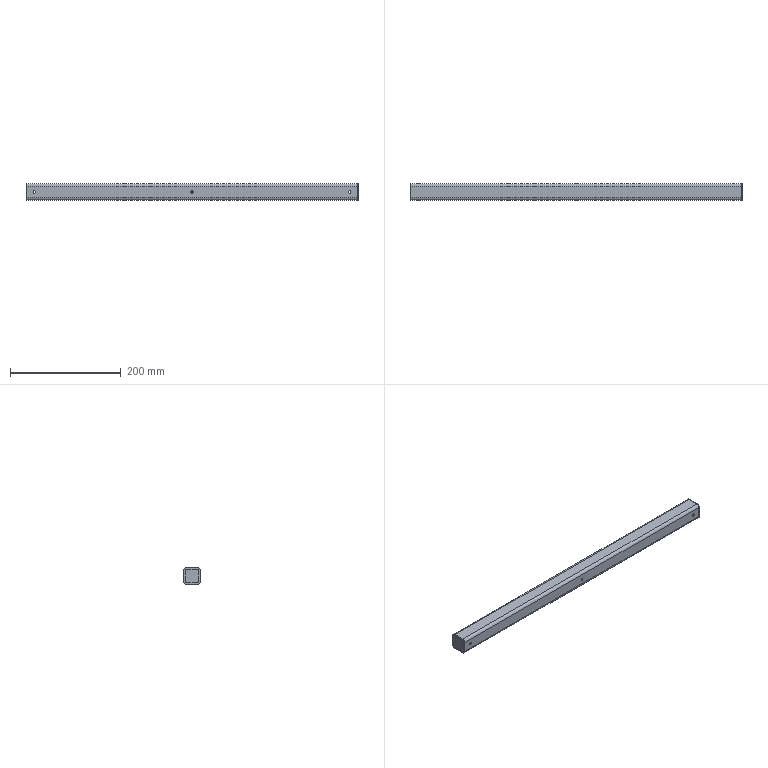Part | SolidWorks | features ICE 2, 3DProfileFeature 1, HoleWzd 1, WeldMemberFeat 1, WeldmentFeature 1 | 3 solids | 50 faces | box 600 x 30 x 30 mm | volume 162072 mm3 | cylinder 28 | plane 22 | commonest cylinder face diameters 4.2 x12 10 x8 5.2 x4 10.4 x4
STEP:
#1=CARTESIAN_POINT('',(0.,-10.,-15.));
#2=VERTEX_POINT('',#1);
#3=CARTESIAN_POINT('',(0.,-15.,-10.));
#4=VERTEX_POINT('',#3);
#5=CARTESIAN_POINT('',(0.,-10.,-10.));
#6=DIRECTION('',(-1.,0.,0.));
#7=DIRECTION('',(0.,0.,-1.));
#8=AXIS2_PLACEMENT_3D('',#5,#6,#7);
#9=CIRCLE('',#8,5.);
#10=EDGE_CURVE('',#2,#4,#9,.T.);
#11=ORIENTED_EDGE('',*,*,#10,.F.);
#12=CARTESIAN_POINT('',(1.,-10.,-15.));
#13=VERTEX_POINT('',#12);
#14=CARTESIAN_POINT('',(1.,-10.,-15.));
#15=DIRECTION('',(-1.,0.,0.));
#16=VECTOR('',#15,1000.);
#17=LINE('',#14,#16);
#18=EDGE_CURVE('',#13,#2,#17,.T.);
#19=ORIENTED_EDGE('',*,*,#18,.F.);
#20=CARTESIAN_POINT('',(1.,-15.,-10.));
#21=VERTEX_POINT('',#20);
#22=CARTESIAN_POINT('',(1.,-10.,-10.));
#23=DIRECTION('',(-1.,0.,0.));
#24=DIRECTION('',(0.,0.,-1.));
#25=AXIS2_PLACEMENT_3D('',#22,#23,#24);
#26=CIRCLE('',#25,5.);
#27=EDGE_CURVE('',#13,#21,#26,.T.);
#28=ORIENTED_EDGE('',*,*,#27,.T.);
#29=CARTESIAN_POINT('',(1.,-15.,-10.));
#30=DIRECTION('',(-1.,0.,0.));
#31=VECTOR('',#30,1000.);
#32=LINE('',#29,#31);
#33=EDGE_CURVE('',#21,#4,#32,.T.);
#34=ORIENTED_EDGE('',*,*,#33,.T.);
#35=EDGE_LOOP('',(#11,#19,#28,#34));
#36=FACE_OUTER_BOUND('',#35,.T.);
#37=CARTESIAN_POINT('',(1.,-10.,-10.));
#38=DIRECTION('',(-1.,0.,0.));
#39=DIRECTION('',(0.,0.,1.));
#40=AXIS2_PLACEMENT_3D('',#37,#38,#39);
#41=CYLINDRICAL_SURFACE('',#40,5.);
#42=ADVANCED_FACE('',(#36),#41,.T.);
#43=CARTESIAN_POINT('',(0.,10.,-15.));
#44=VERTEX_POINT('',#43);
#45=CARTESIAN_POINT('',(0.,10.,-15.));
#46=DIRECTION('',(0.,-1.,0.));
#47=VECTOR('',#46,1000.);
#48=LINE('',#45,#47);
#49=EDGE_CURVE('',#44,#2,#48,.T.);
#50=ORIENTED_EDGE('',*,*,#49,.F.);
#51=CARTESIAN_POINT('',(1.,10.,-15.));
#52=VERTEX_POINT('',#51);
#53=CARTESIAN_POINT('',(1.,10.,-15.));
#54=DIRECTION('',(-1.,0.,0.));
#55=VECTOR('',#54,1000.);
#56=LINE('',#53,#55);
#57=EDGE_CURVE('',#52,#44,#56,.T.);
#58=ORIENTED_EDGE('',*,*,#57,.F.);
#59=CARTESIAN_POINT('',(1.,10.,-15.));
#60=DIRECTION('',(0.,-1.,0.));
#61=VECTOR('',#60,1000.);
#62=LINE('',#59,#61);
#63=EDGE_CURVE('',#52,#13,#62,.T.);
#64=ORIENTED_EDGE('',*,*,#63,.T.);
#65=ORIENTED_EDGE('',*,*,#18,.T.);
#66=EDGE_LOOP('',(#50,#58,#64,#65));
#67=FACE_OUTER_BOUND('',#66,.T.);
#68=CARTESIAN_POINT('',(1.,10.,-15.));
#69=DIRECTION('',(0.,0.,-1.));
#70=DIRECTION('',(-1.,0.,0.));
#71=AXIS2_PLACEMENT_3D('',#68,#69,#70);
#72=PLANE('',#71);
#73=ADVANCED_FACE('',(#67),#72,.T.);
#74=CARTESIAN_POINT('',(0.,15.,-10.));
#75=VERTEX_POINT('',#74);
#76=CARTESIAN_POINT('',(0.,10.,-10.));
#77=DIRECTION('',(-1.,0.,0.));
#78=DIRECTION('',(0.,0.,1.));
#79=AXIS2_PLACEMENT_3D('',#76,#77,#78);
#80=CIRCLE('',#79,5.);
#81=EDGE_CURVE('',#75,#44,#80,.T.);
#82=ORIENTED_EDGE('',*,*,#81,.F.);
#83=CARTESIAN_POINT('',(1.,15.,-10.));
#84=VERTEX_POINT('',#83);
#85=CARTESIAN_POINT('',(1.,15.,-10.));
#86=DIRECTION('',(-1.,0.,0.));
#87=VECTOR('',#86,1000.);
#88=LINE('',#85,#87);
#89=EDGE_CURVE('',#84,#75,#88,.T.);
#90=ORIENTED_EDGE('',*,*,#89,.F.);
#91=CARTESIAN_POINT('',(1.,10.,-10.));
#92=DIRECTION('',(-1.,0.,0.));
#93=DIRECTION('',(0.,0.,1.));
#94=AXIS2_PLACEMENT_3D('',#91,#92,#93);
#95=CIRCLE('',#94,5.);
#96=EDGE_CURVE('',#84,#52,#95,.T.);
#97=ORIENTED_EDGE('',*,*,#96,.T.);
#98=ORIENTED_EDGE('',*,*,#57,.T.);
#99=EDGE_LOOP('',(#82,#90,#97,#98));
#100=FACE_OUTER_BOUND('',#99,.T.);
#101=CARTESIAN_POINT('',(1.,10.,-10.));
#102=DIRECTION('',(-1.,0.,0.));
#103=DIRECTION('',(0.,0.,1.));
#104=AXIS2_PLACEMENT_3D('',#101,#102,#103);
#105=CYLINDRICAL_SURFACE('',#104,5.);
#106=ADVANCED_FACE('',(#100),#105,.T.);
#107=CARTESIAN_POINT('',(0.,15.,10.));
#108=VERTEX_POINT('',#107);
#109=CARTESIAN_POINT('',(0.,15.,10.));
#110=DIRECTION('',(0.,0.,-1.));
#111=VECTOR('',#110,1000.);
#112=LINE('',#109,#111);
#113=EDGE_CURVE('',#108,#75,#112,.T.);
#114=ORIENTED_EDGE('',*,*,#113,.F.);
#115=CARTESIAN_POINT('',(1.,15.,10.));
#116=VERTEX_POINT('',#115);
#117=CARTESIAN_POINT('',(1.,15.,10.));
#118=DIRECTION('',(-1.,0.,0.));
#119=VECTOR('',#118,1000.);
#120=LINE('',#117,#119);
#121=EDGE_CURVE('',#116,#108,#120,.T.);
#122=ORIENTED_EDGE('',*,*,#121,.F.);
#123=CARTESIAN_POINT('',(1.,15.,10.));
#124=DIRECTION('',(0.,0.,-1.));
#125=VECTOR('',#124,1000.);
#126=LINE('',#123,#125);
#127=EDGE_CURVE('',#116,#84,#126,.T.);
#128=ORIENTED_EDGE('',*,*,#127,.T.);
#129=ORIENTED_EDGE('',*,*,#89,.T.);
#130=EDGE_LOOP('',(#114,#122,#128,#129));
#131=FACE_OUTER_BOUND('',#130,.T.);
#132=CARTESIAN_POINT('',(1.,15.,10.));
#133=DIRECTION('',(0.,1.,0.));
#134=DIRECTION('',(0.,0.,1.));
#135=AXIS2_PLACEMENT_3D('',#132,#133,#134);
#136=PLANE('',#135);
#137=ADVANCED_FACE('',(#131),#136,.T.);
#138=CARTESIAN_POINT('',(0.,10.,15.));
#139=VERTEX_POINT('',#138);
#140=CARTESIAN_POINT('',(0.,10.,10.));
#141=DIRECTION('',(-1.,0.,0.));
#142=DIRECTION('',(0.,0.,-1.));
#143=AXIS2_PLACEMENT_3D('',#140,#141,#142);
#144=CIRCLE('',#143,5.);
#145=EDGE_CURVE('',#139,#108,#144,.T.);
#146=ORIENTED_EDGE('',*,*,#145,.F.);
#147=CARTESIAN_POINT('',(1.,10.,15.));
#148=VERTEX_POINT('',#147);
#149=CARTESIAN_POINT('',(1.,10.,15.));
#150=DIRECTION('',(-1.,0.,0.));
#151=VECTOR('',#150,1000.);
#152=LINE('',#149,#151);
#153=EDGE_CURVE('',#148,#139,#152,.T.);
#154=ORIENTED_EDGE('',*,*,#153,.F.);
#155=CARTESIAN_POINT('',(1.,10.,10.));
#156=DIRECTION('',(-1.,0.,0.));
#157=DIRECTION('',(0.,0.,-1.));
#158=AXIS2_PLACEMENT_3D('',#155,#156,#157);
#159=CIRCLE('',#158,5.);
#160=EDGE_CURVE('',#148,#116,#159,.T.);
#161=ORIENTED_EDGE('',*,*,#160,.T.);
#162=ORIENTED_EDGE('',*,*,#121,.T.);
#163=EDGE_LOOP('',(#146,#154,#161,#162));
#164=FACE_OUTER_BOUND('',#163,.T.);
#165=CARTESIAN_POINT('',(1.,10.,10.));
#166=DIRECTION('',(-1.,0.,0.));
#167=DIRECTION('',(0.,0.,1.));
#168=AXIS2_PLACEMENT_3D('',#165,#166,#167);
#169=CYLINDRICAL_SURFACE('',#168,5.);
#170=ADVANCED_FACE('',(#164),#169,.T.);
#171=CARTESIAN_POINT('',(0.,-10.,15.));
#172=VERTEX_POINT('',#171);
#173=CARTESIAN_POINT('',(0.,10.,15.));
#174=DIRECTION('',(0.,1.,0.));
#175=VECTOR('',#174,1000.);
#176=LINE('',#173,#175);
#177=EDGE_CURVE('',#172,#139,#176,.T.);
#178=ORIENTED_EDGE('',*,*,#177,.F.);
#179=CARTESIAN_POINT('',(1.,-10.,15.));
#180=VERTEX_POINT('',#179);
#181=CARTESIAN_POINT('',(1.,-10.,15.));
#182=DIRECTION('',(-1.,0.,0.));
#183=VECTOR('',#182,1000.);
#184=LINE('',#181,#183);
#185=EDGE_CURVE('',#180,#172,#184,.T.);
#186=ORIENTED_EDGE('',*,*,#185,.F.);
#187=CARTESIAN_POINT('',(1.,10.,15.));
#188=DIRECTION('',(0.,1.,0.));
#189=VECTOR('',#188,1000.);
#190=LINE('',#187,#189);
#191=EDGE_CURVE('',#180,#148,#190,.T.);
#192=ORIENTED_EDGE('',*,*,#191,.T.);
#193=ORIENTED_EDGE('',*,*,#153,.T.);
#194=EDGE_LOOP('',(#178,#186,#192,#193));
#195=FACE_OUTER_BOUND('',#194,.T.);
#196=CARTESIAN_POINT('',(1.,10.,15.));
#197=DIRECTION('',(0.,0.,1.));
#198=DIRECTION('',(1.,0.,0.));
#199=AXIS2_PLACEMENT_3D('',#196,#197,#198);
#200=PLANE('',#199);
#201=ADVANCED_FACE('',(#195),#200,.T.);
#202=CARTESIAN_POINT('',(0.,-15.,10.));
#203=VERTEX_POINT('',#202);
#204=CARTESIAN_POINT('',(0.,-10.,10.));
#205=DIRECTION('',(-1.,0.,0.));
#206=DIRECTION('',(0.,0.,-1.));
#207=AXIS2_PLACEMENT_3D('',#204,#205,#206);
#208=CIRCLE('',#207,5.);
#209=EDGE_CURVE('',#203,#172,#208,.T.);
#210=ORIENTED_EDGE('',*,*,#209,.F.);
#211=CARTESIAN_POINT('',(1.,-15.,10.));
#212=VERTEX_POINT('',#211);
#213=CARTESIAN_POINT('',(1.,-15.,10.));
#214=DIRECTION('',(-1.,0.,0.));
#215=VECTOR('',#214,1000.);
#216=LINE('',#213,#215);
#217=EDGE_CURVE('',#212,#203,#216,.T.);
#218=ORIENTED_EDGE('',*,*,#217,.F.);
#219=CARTESIAN_POINT('',(1.,-10.,10.));
#220=DIRECTION('',(-1.,0.,0.));
#221=DIRECTION('',(0.,0.,-1.));
#222=AXIS2_PLACEMENT_3D('',#219,#220,#221);
#223=CIRCLE('',#222,5.);
#224=EDGE_CURVE('',#212,#180,#223,.T.);
#225=ORIENTED_EDGE('',*,*,#224,.T.);
#226=ORIENTED_EDGE('',*,*,#185,.T.);
#227=EDGE_LOOP('',(#210,#218,#225,#226));
#228=FACE_OUTER_BOUND('',#227,.T.);
#229=CARTESIAN_POINT('',(1.,-10.,10.));
#230=DIRECTION('',(-1.,0.,0.));
#231=DIRECTION('',(0.,0.,1.));
#232=AXIS2_PLACEMENT_3D('',#229,#230,#231);
#233=CYLINDRICAL_SURFACE('',#232,5.);
#234=ADVANCED_FACE('',(#228),#233,.T.);
#235=CARTESIAN_POINT('',(0.,-15.,10.));
#236=DIRECTION('',(0.,0.,1.));
#237=VECTOR('',#236,1000.);
#238=LINE('',#235,#237);
#239=EDGE_CURVE('',#4,#203,#238,.T.);
#240=ORIENTED_EDGE('',*,*,#239,.F.);
#241=ORIENTED_EDGE('',*,*,#33,.F.);
#242=CARTESIAN_POINT('',(1.,-15.,10.));
#243=DIRECTION('',(0.,0.,1.));
#244=VECTOR('',#243,1000.);
#245=LINE('',#242,#244);
#246=EDGE_CURVE('',#21,#212,#245,.T.);
#247=ORIENTED_EDGE('',*,*,#246,.T.);
#248=ORIENTED_EDGE('',*,*,#217,.T.);
#249=EDGE_LOOP('',(#240,#241,#247,#248));
#250=FACE_OUTER_BOUND('',#249,.T.);
#251=CARTESIAN_POINT('',(1.,-15.,10.));
#252=DIRECTION('',(0.,-1.,0.));
#253=DIRECTION('',(0.,0.,-1.));
#254=AXIS2_PLACEMENT_3D('',#251,#252,#253);
#255=PLANE('',#254);
#256=ADVANCED_FACE('',(#250),#255,.T.);
#257=ORIENTED_EDGE('',*,*,#27,.F.);
#258=ORIENTED_EDGE('',*,*,#63,.F.);
#259=ORIENTED_EDGE('',*,*,#96,.F.);
#260=ORIENTED_EDGE('',*,*,#127,.F.);
#261=ORIENTED_EDGE('',*,*,#160,.F.);
#262=ORIENTED_EDGE('',*,*,#191,.F.);
#263=ORIENTED_EDGE('',*,*,#224,.F.);
#264=ORIENTED_EDGE('',*,*,#246,.F.);
#265=EDGE_LOOP('',(#257,#258,#259,#260,#261,#262,#263,#264));
#266=FACE_OUTER_BOUND('',#265,.T.);
#267=CARTESIAN_POINT('',(1.,-10.,-10.));
#268=DIRECTION('',(1.,0.,0.));
#269=DIRECTION('',(0.,0.,-1.));
#270=AXIS2_PLACEMENT_3D('',#267,#268,#269);
#271=PLANE('',#270);
#272=ADVANCED_FACE('',(#266),#271,.T.);
#273=ORIENTED_EDGE('',*,*,#10,.T.);
#274=ORIENTED_EDGE('',*,*,#239,.T.);
#275=ORIENTED_EDGE('',*,*,#209,.T.);
#276=ORIENTED_EDGE('',*,*,#177,.T.);
#277=ORIENTED_EDGE('',*,*,#145,.T.);
#278=ORIENTED_EDGE('',*,*,#113,.T.);
#279=ORIENTED_EDGE('',*,*,#81,.T.);
#280=ORIENTED_EDGE('',*,*,#49,.T.);
#281=EDGE_LOOP('',(#273,#274,#275,#276,#277,#278,#279,#280));
#282=FACE_OUTER_BOUND('',#281,.T.);
#283=CARTESIAN_POINT('',(0.,-10.,-10.));
#284=DIRECTION('',(1.,0.,0.));
#285=DIRECTION('',(0.,0.,-1.));
#286=AXIS2_PLACEMENT_3D('',#283,#284,#285);
#287=PLANE('',#286);
#288=ADVANCED_FACE('',(#282),#287,.F.);
#289=CLOSED_SHELL('',(#42,#73,#106,#137,#170,#201,#234,#256,#272,#288));
#290=MANIFOLD_SOLID_BREP('',#289);
#291=CARTESIAN_POINT('',(600.,-10.,15.));
#292=VERTEX_POINT('',#291);
#293=CARTESIAN_POINT('',(600.,-15.,10.));
#294=VERTEX_POINT('',#293);
#295=CARTESIAN_POINT('',(600.,-10.,10.));
#296=DIRECTION('',(1.,0.,0.));
#297=DIRECTION('',(0.,0.,1.));
#298=AXIS2_PLACEMENT_3D('',#295,#296,#297);
#299=CIRCLE('',#298,5.);
#300=EDGE_CURVE('',#292,#294,#299,.T.);
#301=ORIENTED_EDGE('',*,*,#300,.F.);
#302=CARTESIAN_POINT('',(599.,-10.,15.));
#303=VERTEX_POINT('',#302);
#304=CARTESIAN_POINT('',(599.,-10.,15.));
#305=DIRECTION('',(1.,0.,0.));
#306=VECTOR('',#305,1000.);
#307=LINE('',#304,#306);
#308=EDGE_CURVE('',#303,#292,#307,.T.);
#309=ORIENTED_EDGE('',*,*,#308,.F.);
#310=CARTESIAN_POINT('',(599.,-15.,10.));
#311=VERTEX_POINT('',#310);
#312=CARTESIAN_POINT('',(599.,-10.,10.));
#313=DIRECTION('',(1.,0.,0.));
#314=DIRECTION('',(0.,0.,1.));
#315=AXIS2_PLACEMENT_3D('',#312,#313,#314);
#316=CIRCLE('',#315,5.);
#317=EDGE_CURVE('',#303,#311,#316,.T.);
#318=ORIENTED_EDGE('',*,*,#317,.T.);
#319=CARTESIAN_POINT('',(599.,-15.,10.));
#320=DIRECTION('',(1.,0.,0.));
#321=VECTOR('',#320,1000.);
#322=LINE('',#319,#321);
#323=EDGE_CURVE('',#311,#294,#322,.T.);
#324=ORIENTED_EDGE('',*,*,#323,.T.);
#325=EDGE_LOOP('',(#301,#309,#318,#324));
#326=FACE_OUTER_BOUND('',#325,.T.);
#327=CARTESIAN_POINT('',(599.,-10.,10.));
#328=DIRECTION('',(1.,0.,0.));
#329=DIRECTION('',(0.,0.,-1.));
#330=AXIS2_PLACEMENT_3D('',#327,#328,#329);
#331=CYLINDRICAL_SURFACE('',#330,5.);
#332=ADVANCED_FACE('',(#326),#331,.T.);
#333=CARTESIAN_POINT('',(600.,10.,15.));
#334=VERTEX_POINT('',#333);
#335=CARTESIAN_POINT('',(600.,10.,15.));
#336=DIRECTION('',(0.,-1.,0.));
#337=VECTOR('',#336,1000.);
#338=LINE('',#335,#337);
#339=EDGE_CURVE('',#334,#292,#338,.T.);
#340=ORIENTED_EDGE('',*,*,#339,.F.);
#341=CARTESIAN_POINT('',(599.,10.,15.));
#342=VERTEX_POINT('',#341);
#343=CARTESIAN_POINT('',(599.,10.,15.));
#344=DIRECTION('',(1.,0.,0.));
#345=VECTOR('',#344,1000.);
#346=LINE('',#343,#345);
#347=EDGE_CURVE('',#342,#334,#346,.T.);
#348=ORIENTED_EDGE('',*,*,#347,.F.);
#349=CARTESIAN_POINT('',(599.,10.,15.));
#350=DIRECTION('',(0.,-1.,0.));
#351=VECTOR('',#350,1000.);
#352=LINE('',#349,#351);
#353=EDGE_CURVE('',#342,#303,#352,.T.);
#354=ORIENTED_EDGE('',*,*,#353,.T.);
#355=ORIENTED_EDGE('',*,*,#308,.T.);
#356=EDGE_LOOP('',(#340,#348,#354,#355));
#357=FACE_OUTER_BOUND('',#356,.T.);
#358=CARTESIAN_POINT('',(599.,10.,15.));
#359=DIRECTION('',(0.,0.,1.));
#360=DIRECTION('',(1.,0.,0.));
#361=AXIS2_PLACEMENT_3D('',#358,#359,#360);
#362=PLANE('',#361);
#363=ADVANCED_FACE('',(#357),#362,.T.);
#364=CARTESIAN_POINT('',(600.,15.,10.));
#365=VERTEX_POINT('',#364);
#366=CARTESIAN_POINT('',(600.,10.,10.));
#367=DIRECTION('',(1.,0.,0.));
#368=DIRECTION('',(0.,0.,-1.));
#369=AXIS2_PLACEMENT_3D('',#366,#367,#368);
#370=CIRCLE('',#369,5.);
#371=EDGE_CURVE('',#365,#334,#370,.T.);
#372=ORIENTED_EDGE('',*,*,#371,.F.);
#373=CARTESIAN_POINT('',(599.,15.,10.));
#374=VERTEX_POINT('',#373);
#375=CARTESIAN_POINT('',(599.,15.,10.));
#376=DIRECTION('',(1.,0.,0.));
#377=VECTOR('',#376,1000.);
#378=LINE('',#375,#377);
#379=EDGE_CURVE('',#374,#365,#378,.T.);
#380=ORIENTED_EDGE('',*,*,#379,.F.);
#381=CARTESIAN_POINT('',(599.,10.,10.));
#382=DIRECTION('',(1.,0.,0.));
#383=DIRECTION('',(0.,0.,-1.));
#384=AXIS2_PLACEMENT_3D('',#381,#382,#383);
#385=CIRCLE('',#384,5.);
#386=EDGE_CURVE('',#374,#342,#385,.T.);
#387=ORIENTED_EDGE('',*,*,#386,.T.);
#388=ORIENTED_EDGE('',*,*,#347,.T.);
#389=EDGE_LOOP('',(#372,#380,#387,#388));
#390=FACE_OUTER_BOUND('',#389,.T.);
#391=CARTESIAN_POINT('',(599.,10.,10.));
#392=DIRECTION('',(1.,0.,0.));
#393=DIRECTION('',(0.,0.,-1.));
#394=AXIS2_PLACEMENT_3D('',#391,#392,#393);
#395=CYLINDRICAL_SURFACE('',#394,5.);
#396=ADVANCED_FACE('',(#390),#395,.T.);
#397=CARTESIAN_POINT('',(600.,15.,-10.));
#398=VERTEX_POINT('',#397);
#399=CARTESIAN_POINT('',(600.,15.,-10.));
#400=DIRECTION('',(0.,0.,1.));
#401=VECTOR('',#400,1000.);
#402=LINE('',#399,#401);
#403=EDGE_CURVE('',#398,#365,#402,.T.);
#404=ORIENTED_EDGE('',*,*,#403,.F.);
#405=CARTESIAN_POINT('',(599.,15.,-10.));
#406=VERTEX_POINT('',#405);
#407=CARTESIAN_POINT('',(599.,15.,-10.));
#408=DIRECTION('',(1.,0.,0.));
#409=VECTOR('',#408,1000.);
#410=LINE('',#407,#409);
#411=EDGE_CURVE('',#406,#398,#410,.T.);
#412=ORIENTED_EDGE('',*,*,#411,.F.);
#413=CARTESIAN_POINT('',(599.,15.,-10.));
#414=DIRECTION('',(0.,0.,1.));
#415=VECTOR('',#414,1000.);
#416=LINE('',#413,#415);
#417=EDGE_CURVE('',#406,#374,#416,.T.);
#418=ORIENTED_EDGE('',*,*,#417,.T.);
#419=ORIENTED_EDGE('',*,*,#379,.T.);
#420=EDGE_LOOP('',(#404,#412,#418,#419));
#421=FACE_OUTER_BOUND('',#420,.T.);
#422=CARTESIAN_POINT('',(599.,15.,-10.));
#423=DIRECTION('',(0.,1.,0.));
#424=DIRECTION('',(0.,0.,1.));
#425=AXIS2_PLACEMENT_3D('',#422,#423,#424);
#426=PLANE('',#425);
#427=ADVANCED_FACE('',(#421),#426,.T.);
#428=CARTESIAN_POINT('',(600.,10.,-15.));
#429=VERTEX_POINT('',#428);
#430=CARTESIAN_POINT('',(600.,10.,-10.));
#431=DIRECTION('',(1.,0.,0.));
#432=DIRECTION('',(0.,0.,1.));
#433=AXIS2_PLACEMENT_3D('',#430,#431,#432);
#434=CIRCLE('',#433,5.);
#435=EDGE_CURVE('',#429,#398,#434,.T.);
#436=ORIENTED_EDGE('',*,*,#435,.F.);
#437=CARTESIAN_POINT('',(599.,10.,-15.));
#438=VERTEX_POINT('',#437);
#439=CARTESIAN_POINT('',(599.,10.,-15.));
#440=DIRECTION('',(1.,0.,0.));
#441=VECTOR('',#440,1000.);
#442=LINE('',#439,#441);
#443=EDGE_CURVE('',#438,#429,#442,.T.);
#444=ORIENTED_EDGE('',*,*,#443,.F.);
#445=CARTESIAN_POINT('',(599.,10.,-10.));
#446=DIRECTION('',(1.,0.,0.));
#447=DIRECTION('',(0.,0.,1.));
#448=AXIS2_PLACEMENT_3D('',#445,#446,#447);
#449=CIRCLE('',#448,5.);
#450=EDGE_CURVE('',#438,#406,#449,.T.);
#451=ORIENTED_EDGE('',*,*,#450,.T.);
#452=ORIENTED_EDGE('',*,*,#411,.T.);
#453=EDGE_LOOP('',(#436,#444,#451,#452));
#454=FACE_OUTER_BOUND('',#453,.T.);
#455=CARTESIAN_POINT('',(599.,10.,-10.));
#456=DIRECTION('',(1.,0.,0.));
#457=DIRECTION('',(0.,0.,-1.));
#458=AXIS2_PLACEMENT_3D('',#455,#456,#457);
#459=CYLINDRICAL_SURFACE('',#458,5.);
#460=ADVANCED_FACE('',(#454),#459,.T.);
#461=CARTESIAN_POINT('',(600.,-10.,-15.));
#462=VERTEX_POINT('',#461);
#463=CARTESIAN_POINT('',(600.,10.,-15.));
#464=DIRECTION('',(0.,1.,0.));
#465=VECTOR('',#464,1000.);
#466=LINE('',#463,#465);
#467=EDGE_CURVE('',#462,#429,#466,.T.);
#468=ORIENTED_EDGE('',*,*,#467,.F.);
#469=CARTESIAN_POINT('',(599.,-10.,-15.));
#470=VERTEX_POINT('',#469);
#471=CARTESIAN_POINT('',(599.,-10.,-15.));
#472=DIRECTION('',(1.,0.,0.));
#473=VECTOR('',#472,1000.);
#474=LINE('',#471,#473);
#475=EDGE_CURVE('',#470,#462,#474,.T.);
#476=ORIENTED_EDGE('',*,*,#475,.F.);
#477=CARTESIAN_POINT('',(599.,10.,-15.));
#478=DIRECTION('',(0.,1.,0.));
#479=VECTOR('',#478,1000.);
#480=LINE('',#477,#479);
#481=EDGE_CURVE('',#470,#438,#480,.T.);
#482=ORIENTED_EDGE('',*,*,#481,.T.);
#483=ORIENTED_EDGE('',*,*,#443,.T.);
#484=EDGE_LOOP('',(#468,#476,#482,#483));
#485=FACE_OUTER_BOUND('',#484,.T.);
#486=CARTESIAN_POINT('',(599.,10.,-15.));
#487=DIRECTION('',(0.,0.,-1.));
#488=DIRECTION('',(-1.,0.,0.));
#489=AXIS2_PLACEMENT_3D('',#486,#487,#488);
#490=PLANE('',#489);
#491=ADVANCED_FACE('',(#485),#490,.T.);
#492=CARTESIAN_POINT('',(600.,-15.,-10.));
#493=VERTEX_POINT('',#492);
#494=CARTESIAN_POINT('',(600.,-10.,-10.));
#495=DIRECTION('',(1.,0.,0.));
#496=DIRECTION('',(0.,0.,1.));
#497=AXIS2_PLACEMENT_3D('',#494,#495,#496);
#498=CIRCLE('',#497,5.);
#499=EDGE_CURVE('',#493,#462,#498,.T.);
#500=ORIENTED_EDGE('',*,*,#499,.F.);
#501=CARTESIAN_POINT('',(599.,-15.,-10.));
#502=VERTEX_POINT('',#501);
#503=CARTESIAN_POINT('',(599.,-15.,-10.));
#504=DIRECTION('',(1.,0.,0.));
#505=VECTOR('',#504,1000.);
#506=LINE('',#503,#505);
#507=EDGE_CURVE('',#502,#493,#506,.T.);
#508=ORIENTED_EDGE('',*,*,#507,.F.);
#509=CARTESIAN_POINT('',(599.,-10.,-10.));
#510=DIRECTION('',(1.,0.,0.));
#511=DIRECTION('',(0.,0.,1.));
#512=AXIS2_PLACEMENT_3D('',#509,#510,#511);
#513=CIRCLE('',#512,5.);
#514=EDGE_CURVE('',#502,#470,#513,.T.);
#515=ORIENTED_EDGE('',*,*,#514,.T.);
#516=ORIENTED_EDGE('',*,*,#475,.T.);
#517=EDGE_LOOP('',(#500,#508,#515,#516));
#518=FACE_OUTER_BOUND('',#517,.T.);
#519=CARTESIAN_POINT('',(599.,-10.,-10.));
#520=DIRECTION('',(1.,0.,0.));
#521=DIRECTION('',(0.,0.,-1.));
#522=AXIS2_PLACEMENT_3D('',#519,#520,#521);
#523=CYLINDRICAL_SURFACE('',#522,5.);
#524=ADVANCED_FACE('',(#518),#523,.T.);
#525=CARTESIAN_POINT('',(600.,-15.,-10.));
#526=DIRECTION('',(0.,0.,-1.));
#527=VECTOR('',#526,1000.);
#528=LINE('',#525,#527);
#529=EDGE_CURVE('',#294,#493,#528,.T.);
#530=ORIENTED_EDGE('',*,*,#529,.F.);
#531=ORIENTED_EDGE('',*,*,#323,.F.);
#532=CARTESIAN_POINT('',(599.,-15.,-10.));
#533=DIRECTION('',(0.,0.,-1.));
#534=VECTOR('',#533,1000.);
#535=LINE('',#532,#534);
#536=EDGE_CURVE('',#311,#502,#535,.T.);
#537=ORIENTED_EDGE('',*,*,#536,.T.);
#538=ORIENTED_EDGE('',*,*,#507,.T.);
#539=EDGE_LOOP('',(#530,#531,#537,#538));
#540=FACE_OUTER_BOUND('',#539,.T.);
#541=CARTESIAN_POINT('',(599.,-15.,-10.));
#542=DIRECTION('',(0.,-1.,0.));
#543=DIRECTION('',(0.,0.,-1.));
#544=AXIS2_PLACEMENT_3D('',#541,#542,#543);
#545=PLANE('',#544);
#546=ADVANCED_FACE('',(#540),#545,.T.);
#547=ORIENTED_EDGE('',*,*,#317,.F.);
#548=ORIENTED_EDGE('',*,*,#353,.F.);
#549=ORIENTED_EDGE('',*,*,#386,.F.);
#550=ORIENTED_EDGE('',*,*,#417,.F.);
#551=ORIENTED_EDGE('',*,*,#450,.F.);
#552=ORIENTED_EDGE('',*,*,#481,.F.);
#553=ORIENTED_EDGE('',*,*,#514,.F.);
#554=ORIENTED_EDGE('',*,*,#536,.F.);
#555=EDGE_LOOP('',(#547,#548,#549,#550,#551,#552,#553,#554));
#556=FACE_OUTER_BOUND('',#555,.T.);
#557=CARTESIAN_POINT('',(599.,-10.,10.));
#558=DIRECTION('',(-1.,0.,0.));
#559=DIRECTION('',(0.,0.,1.));
#560=AXIS2_PLACEMENT_3D('',#557,#558,#559);
#561=PLANE('',#560);
#562=ADVANCED_FACE('',(#556),#561,.T.);
#563=ORIENTED_EDGE('',*,*,#300,.T.);
#564=ORIENTED_EDGE('',*,*,#529,.T.);
#565=ORIENTED_EDGE('',*,*,#499,.T.);
#566=ORIENTED_EDGE('',*,*,#467,.T.);
#567=ORIENTED_EDGE('',*,*,#435,.T.);
#568=ORIENTED_EDGE('',*,*,#403,.T.);
#569=ORIENTED_EDGE('',*,*,#371,.T.);
#570=ORIENTED_EDGE('',*,*,#339,.T.);
#571=EDGE_LOOP('',(#563,#564,#565,#566,#567,#568,#569,#570));
#572=FACE_OUTER_BOUND('',#571,.T.);
#573=CARTESIAN_POINT('',(600.,-10.,10.));
#574=DIRECTION('',(-1.,0.,0.));
#575=DIRECTION('',(0.,0.,1.));
#576=AXIS2_PLACEMENT_3D('',#573,#574,#575);
#577=PLANE('',#576);
#578=ADVANCED_FACE('',(#572),#577,.F.);
#579=CLOSED_SHELL('',(#332,#363,#396,#427,#460,#491,#524,#546,#562,#578));
#580=MANIFOLD_SOLID_BREP('',#579);
#581=CARTESIAN_POINT('',(15.,15.,2.1));
#582=VERTEX_POINT('',#581);
#583=CARTESIAN_POINT('',(15.,15.,-2.1));
#584=VERTEX_POINT('',#583);
#585=CARTESIAN_POINT('',(15.,15.,0.000000001));
#586=DIRECTION('',(0.,-1.,0.));
#587=DIRECTION('',(0.,0.,-1.));
#588=AXIS2_PLACEMENT_3D('',#585,#586,#587);
#589=CIRCLE('',#588,2.1);
#590=EDGE_CURVE('',#582,#584,#589,.T.);
#591=ORIENTED_EDGE('',*,*,#590,.F.);
#592=CARTESIAN_POINT('',(15.,12.4,2.1));
#593=VERTEX_POINT('',#592);
#594=CARTESIAN_POINT('',(15.,-15.,2.1));
#595=DIRECTION('',(0.,-1.,0.));
#596=VECTOR('',#595,1000.);
#597=LINE('',#594,#596);
#598=EDGE_CURVE('',#582,#593,#597,.T.);
#599=ORIENTED_EDGE('',*,*,#598,.T.);
#600=CARTESIAN_POINT('',(15.,12.4,-2.1));
#601=VERTEX_POINT('',#600);
#602=CARTESIAN_POINT('',(15.,12.4,0.000000001));
#603=DIRECTION('',(0.,-1.,0.));
#604=DIRECTION('',(0.,0.,-1.));
#605=AXIS2_PLACEMENT_3D('',#602,#603,#604);
#606=CIRCLE('',#605,2.1);
#607=EDGE_CURVE('',#593,#601,#606,.T.);
#608=ORIENTED_EDGE('',*,*,#607,.T.);
#609=CARTESIAN_POINT('',(15.,-15.,-2.1));
#610=DIRECTION('',(0.,-1.,0.));
#611=VECTOR('',#610,1000.);
#612=LINE('',#609,#611);
#613=EDGE_CURVE('',#584,#601,#612,.T.);
#614=ORIENTED_EDGE('',*,*,#613,.F.);
#615=EDGE_LOOP('',(#591,#599,#608,#614));
#616=FACE_OUTER_BOUND('',#615,.T.);
#617=CARTESIAN_POINT('',(15.,-15.,0.000000001));
#618=DIRECTION('',(0.,-1.,0.));
#619=DIRECTION('',(0.,0.,-1.));
#620=AXIS2_PLACEMENT_3D('',#617,#618,#619);
#621=CYLINDRICAL_SURFACE('',#620,2.1);
#622=ADVANCED_FACE('',(#616),#621,.F.);
#623=CARTESIAN_POINT('',(15.,-12.4,-2.1));
#624=VERTEX_POINT('',#623);
#625=CARTESIAN_POINT('',(15.,-12.4,2.1));
#626=VERTEX_POINT('',#625);
#627=CARTESIAN_POINT('',(15.,-12.4,0.000000001));
#628=DIRECTION('',(0.,1.,0.));
#629=DIRECTION('',(0.,0.,1.));
#630=AXIS2_PLACEMENT_3D('',#627,#628,#629);
#631=CIRCLE('',#630,2.1);
#632=EDGE_CURVE('',#624,#626,#631,.T.);
#633=ORIENTED_EDGE('',*,*,#632,.T.);
#634=CARTESIAN_POINT('',(15.,-15.,2.1));
#635=VERTEX_POINT('',#634);
#636=CARTESIAN_POINT('',(15.,-15.,2.1));
#637=DIRECTION('',(0.,-1.,0.));
#638=VECTOR('',#637,1000.);
#639=LINE('',#636,#638);
#640=EDGE_CURVE('',#626,#635,#639,.T.);
#641=ORIENTED_EDGE('',*,*,#640,.T.);
#642=CARTESIAN_POINT('',(15.,-15.,-2.1));
#643=VERTEX_POINT('',#642);
#644=CARTESIAN_POINT('',(15.,-15.,0.000000001));
#645=DIRECTION('',(0.,-1.,0.));
#646=DIRECTION('',(0.,0.,-1.));
#647=AXIS2_PLACEMENT_3D('',#644,#645,#646);
#648=CIRCLE('',#647,2.1);
#649=EDGE_CURVE('',#635,#643,#648,.T.);
#650=ORIENTED_EDGE('',*,*,#649,.T.);
#651=CARTESIAN_POINT('',(15.,-15.,-2.1));
#652=DIRECTION('',(0.,-1.,0.));
#653=VECTOR('',#652,1000.);
#654=LINE('',#651,#653);
#655=EDGE_CURVE('',#624,#643,#654,.T.);
#656=ORIENTED_EDGE('',*,*,#655,.F.);
#657=EDGE_LOOP('',(#633,#641,#650,#656));
#658=FACE_OUTER_BOUND('',#657,.T.);
#659=CARTESIAN_POINT('',(15.,-15.,0.000000001));
#660=DIRECTION('',(0.,-1.,0.));
#661=DIRECTION('',(0.,0.,-1.));
#662=AXIS2_PLACEMENT_3D('',#659,#660,#661);
#663=CYLINDRICAL_SURFACE('',#662,2.1);
#664=ADVANCED_FACE('',(#658),#663,.F.);
#665=CARTESIAN_POINT('',(300.,15.,2.1));
#666=VERTEX_POINT('',#665);
#667=CARTESIAN_POINT('',(300.,15.,-2.1));
#668=VERTEX_POINT('',#667);
#669=CARTESIAN_POINT('',(300.,15.,0.000000001));
#670=DIRECTION('',(0.,-1.,0.));
#671=DIRECTION('',(0.,0.,-1.));
#672=AXIS2_PLACEMENT_3D('',#669,#670,#671);
#673=CIRCLE('',#672,2.1);
#674=EDGE_CURVE('',#666,#668,#673,.T.);
#675=ORIENTED_EDGE('',*,*,#674,.F.);
#676=CARTESIAN_POINT('',(300.,12.4,2.1));
#677=VERTEX_POINT('',#676);
#678=CARTESIAN_POINT('',(300.,-15.,2.1));
#679=DIRECTION('',(0.,-1.,0.));
#680=VECTOR('',#679,1000.);
#681=LINE('',#678,#680);
#682=EDGE_CURVE('',#666,#677,#681,.T.);
#683=ORIENTED_EDGE('',*,*,#682,.T.);
#684=CARTESIAN_POINT('',(300.,12.4,-2.1));
#685=VERTEX_POINT('',#684);
#686=CARTESIAN_POINT('',(300.,12.4,0.000000001));
#687=DIRECTION('',(0.,-1.,0.));
#688=DIRECTION('',(0.,0.,-1.));
#689=AXIS2_PLACEMENT_3D('',#686,#687,#688);
#690=CIRCLE('',#689,2.1);
#691=EDGE_CURVE('',#677,#685,#690,.T.);
#692=ORIENTED_EDGE('',*,*,#691,.T.);
#693=CARTESIAN_POINT('',(300.,-15.,-2.1));
#694=DIRECTION('',(0.,-1.,0.));
#695=VECTOR('',#694,1000.);
#696=LINE('',#693,#695);
#697=EDGE_CURVE('',#668,#685,#696,.T.);
#698=ORIENTED_EDGE('',*,*,#697,.F.);
#699=EDGE_LOOP('',(#675,#683,#692,#698));
#700=FACE_OUTER_BOUND('',#699,.T.);
#701=CARTESIAN_POINT('',(300.,-15.,0.000000001));
#702=DIRECTION('',(0.,-1.,0.));
#703=DIRECTION('',(0.,0.,-1.));
#704=AXIS2_PLACEMENT_3D('',#701,#702,#703);
#705=CYLINDRICAL_SURFACE('',#704,2.1);
#706=ADVANCED_FACE('',(#700),#705,.F.);
#707=CARTESIAN_POINT('',(300.,-12.4,-2.1));
#708=VERTEX_POINT('',#707);
#709=CARTESIAN_POINT('',(300.,-12.4,2.1));
#710=VERTEX_POINT('',#709);
#711=CARTESIAN_POINT('',(300.,-12.4,0.000000001));
#712=DIRECTION('',(0.,1.,0.));
#713=DIRECTION('',(0.,0.,1.));
#714=AXIS2_PLACEMENT_3D('',#711,#712,#713);
#715=CIRCLE('',#714,2.1);
#716=EDGE_CURVE('',#708,#710,#715,.T.);
#717=ORIENTED_EDGE('',*,*,#716,.T.);
#718=CARTESIAN_POINT('',(300.,-15.,2.1));
#719=VERTEX_POINT('',#718);
#720=CARTESIAN_POINT('',(300.,-15.,2.1));
#721=DIRECTION('',(0.,-1.,0.));
#722=VECTOR('',#721,1000.);
#723=LINE('',#720,#722);
#724=EDGE_CURVE('',#710,#719,#723,.T.);
#725=ORIENTED_EDGE('',*,*,#724,.T.);
#726=CARTESIAN_POINT('',(300.,-15.,-2.1));
#727=VERTEX_POINT('',#726);
#728=CARTESIAN_POINT('',(300.,-15.,0.000000001));
#729=DIRECTION('',(0.,-1.,0.));
#730=DIRECTION('',(0.,0.,-1.));
#731=AXIS2_PLACEMENT_3D('',#728,#729,#730);
#732=CIRCLE('',#731,2.1);
#733=EDGE_CURVE('',#719,#727,#732,.T.);
#734=ORIENTED_EDGE('',*,*,#733,.T.);
#735=CARTESIAN_POINT('',(300.,-15.,-2.1));
#736=DIRECTION('',(0.,-1.,0.));
#737=VECTOR('',#736,1000.);
#738=LINE('',#735,#737);
#739=EDGE_CURVE('',#708,#727,#738,.T.);
#740=ORIENTED_EDGE('',*,*,#739,.F.);
#741=EDGE_LOOP('',(#717,#725,#734,#740));
#742=FACE_OUTER_BOUND('',#741,.T.);
#743=CARTESIAN_POINT('',(300.,-15.,0.000000001));
#744=DIRECTION('',(0.,-1.,0.));
#745=DIRECTION('',(0.,0.,-1.));
#746=AXIS2_PLACEMENT_3D('',#743,#744,#745);
#747=CYLINDRICAL_SURFACE('',#746,2.1);
#748=ADVANCED_FACE('',(#742),#747,.F.);
#749=CARTESIAN_POINT('',(585.,15.,2.1));
#750=VERTEX_POINT('',#749);
#751=CARTESIAN_POINT('',(585.,15.,-2.1));
#752=VERTEX_POINT('',#751);
#753=CARTESIAN_POINT('',(585.,15.,0.000000001));
#754=DIRECTION('',(0.,-1.,0.));
#755=DIRECTION('',(0.,0.,-1.));
#756=AXIS2_PLACEMENT_3D('',#753,#754,#755);
#757=CIRCLE('',#756,2.1);
#758=EDGE_CURVE('',#750,#752,#757,.T.);
#759=ORIENTED_EDGE('',*,*,#758,.F.);
#760=CARTESIAN_POINT('',(585.,12.4,2.1));
#761=VERTEX_POINT('',#760);
#762=CARTESIAN_POINT('',(585.,-15.,2.1));
#763=DIRECTION('',(0.,-1.,0.));
#764=VECTOR('',#763,1000.);
#765=LINE('',#762,#764);
#766=EDGE_CURVE('',#750,#761,#765,.T.);
#767=ORIENTED_EDGE('',*,*,#766,.T.);
#768=CARTESIAN_POINT('',(585.,12.4,-2.1));
#769=VERTEX_POINT('',#768);
#770=CARTESIAN_POINT('',(585.,12.4,0.000000001));
#771=DIRECTION('',(0.,-1.,0.));
#772=DIRECTION('',(0.,0.,-1.));
#773=AXIS2_PLACEMENT_3D('',#770,#771,#772);
#774=CIRCLE('',#773,2.1);
#775=EDGE_CURVE('',#761,#769,#774,.T.);
#776=ORIENTED_EDGE('',*,*,#775,.T.);
#777=CARTESIAN_POINT('',(585.,-15.,-2.1));
#778=DIRECTION('',(0.,-1.,0.));
#779=VECTOR('',#778,1000.);
#780=LINE('',#777,#779);
#781=EDGE_CURVE('',#752,#769,#780,.T.);
#782=ORIENTED_EDGE('',*,*,#781,.F.);
#783=EDGE_LOOP('',(#759,#767,#776,#782));
#784=FACE_OUTER_BOUND('',#783,.T.);
#785=CARTESIAN_POINT('',(585.,-15.,0.000000001));
#786=DIRECTION('',(0.,-1.,0.));
#787=DIRECTION('',(0.,0.,-1.));
#788=AXIS2_PLACEMENT_3D('',#785,#786,#787);
#789=CYLINDRICAL_SURFACE('',#788,2.1);
#790=ADVANCED_FACE('',(#784),#789,.F.);
#791=CARTESIAN_POINT('',(585.,-12.4,-2.1));
#792=VERTEX_POINT('',#791);
#793=CARTESIAN_POINT('',(585.,-12.4,2.1));
#794=VERTEX_POINT('',#793);
#795=CARTESIAN_POINT('',(585.,-12.4,0.000000001));
#796=DIRECTION('',(0.,1.,0.));
#797=DIRECTION('',(0.,0.,1.));
#798=AXIS2_PLACEMENT_3D('',#795,#796,#797);
#799=CIRCLE('',#798,2.1);
#800=EDGE_CURVE('',#792,#794,#799,.T.);
#801=ORIENTED_EDGE('',*,*,#800,.T.);
#802=CARTESIAN_POINT('',(585.,-15.,2.1));
#803=VERTEX_POINT('',#802);
#804=CARTESIAN_POINT('',(585.,-15.,2.1));
#805=DIRECTION('',(0.,-1.,0.));
#806=VECTOR('',#805,1000.);
#807=LINE('',#804,#806);
#808=EDGE_CURVE('',#794,#803,#807,.T.);
#809=ORIENTED_EDGE('',*,*,#808,.T.);
#810=CARTESIAN_POINT('',(585.,-15.,-2.1));
#811=VERTEX_POINT('',#810);
#812=CARTESIAN_POINT('',(585.,-15.,0.000000001));
#813=DIRECTION('',(0.,-1.,0.));
#814=DIRECTION('',(0.,0.,-1.));
#815=AXIS2_PLACEMENT_3D('',#812,#813,#814);
#816=CIRCLE('',#815,2.1);
#817=EDGE_CURVE('',#803,#811,#816,.T.);
#818=ORIENTED_EDGE('',*,*,#817,.T.);
#819=CARTESIAN_POINT('',(585.,-15.,-2.1));
#820=DIRECTION('',(0.,-1.,0.));
#821=VECTOR('',#820,1000.);
#822=LINE('',#819,#821);
#823=EDGE_CURVE('',#792,#811,#822,.T.);
#824=ORIENTED_EDGE('',*,*,#823,.F.);
#825=EDGE_LOOP('',(#801,#809,#818,#824));
#826=FACE_OUTER_BOUND('',#825,.T.);
#827=CARTESIAN_POINT('',(585.,-15.,0.000000001));
#828=DIRECTION('',(0.,-1.,0.));
#829=DIRECTION('',(0.,0.,-1.));
#830=AXIS2_PLACEMENT_3D('',#827,#828,#829);
#831=CYLINDRICAL_SURFACE('',#830,2.1);
#832=ADVANCED_FACE('',(#826),#831,.F.);
#833=CARTESIAN_POINT('',(0.,9.8,-15.));
#834=VERTEX_POINT('',#833);
#835=CARTESIAN_POINT('',(0.,15.,-9.8));
#836=VERTEX_POINT('',#835);
#837=CARTESIAN_POINT('',(0.,9.8,-9.8));
#838=DIRECTION('',(1.,0.,0.));
#839=DIRECTION('',(0.,0.,-1.));
#840=AXIS2_PLACEMENT_3D('',#837,#838,#839);
#841=CIRCLE('',#840,5.2);
#842=EDGE_CURVE('',#834,#836,#841,.T.);
#843=ORIENTED_EDGE('',*,*,#842,.T.);
#844=CARTESIAN_POINT('',(600.,15.,-9.8));
#845=VERTEX_POINT('',#844);
#846=CARTESIAN_POINT('',(600.,15.,-9.8));
#847=DIRECTION('',(-1.,0.,0.));
#848=VECTOR('',#847,1000.);
#849=LINE('',#846,#848);
#850=EDGE_CURVE('',#845,#836,#849,.T.);
#851=ORIENTED_EDGE('',*,*,#850,.F.);
#852=CARTESIAN_POINT('',(600.,9.8,-15.));
#853=VERTEX_POINT('',#852);
#854=CARTESIAN_POINT('',(600.,9.8,-9.8));
#855=DIRECTION('',(1.,0.,0.));
#856=DIRECTION('',(0.,0.,-1.));
#857=AXIS2_PLACEMENT_3D('',#854,#855,#856);
#858=CIRCLE('',#857,5.2);
#859=EDGE_CURVE('',#853,#845,#858,.T.);
#860=ORIENTED_EDGE('',*,*,#859,.F.);
#861=CARTESIAN_POINT('',(600.,9.8,-15.));
#862=DIRECTION('',(-1.,0.,0.));
#863=VECTOR('',#862,1000.);
#864=LINE('',#861,#863);
#865=EDGE_CURVE('',#853,#834,#864,.T.);
#866=ORIENTED_EDGE('',*,*,#865,.T.);
#867=EDGE_LOOP('',(#843,#851,#860,#866));
#868=FACE_OUTER_BOUND('',#867,.T.);
#869=CARTESIAN_POINT('',(600.,9.8,-9.8));
#870=DIRECTION('',(-1.,0.,0.));
#871=DIRECTION('',(0.,0.,1.));
#872=AXIS2_PLACEMENT_3D('',#869,#870,#871);
#873=CYLINDRICAL_SURFACE('',#872,5.2);
#874=ADVANCED_FACE('',(#868),#873,.T.);
#875=CARTESIAN_POINT('',(15.,15.,0.000000001));
#876=DIRECTION('',(0.,-1.,0.));
#877=DIRECTION('',(0.,0.,-1.));
#878=AXIS2_PLACEMENT_3D('',#875,#876,#877);
#879=CIRCLE('',#878,2.1);
#880=EDGE_CURVE('',#584,#582,#879,.T.);
#881=ORIENTED_EDGE('',*,*,#880,.T.);
#882=ORIENTED_EDGE('',*,*,#590,.T.);
#883=EDGE_LOOP('',(#881,#882));
#884=FACE_BOUND('',#883,.T.);
#885=CARTESIAN_POINT('',(300.,15.,0.000000001));
#886=DIRECTION('',(0.,-1.,0.));
#887=DIRECTION('',(0.,0.,-1.));
#888=AXIS2_PLACEMENT_3D('',#885,#886,#887);
#889=CIRCLE('',#888,2.1);
#890=EDGE_CURVE('',#668,#666,#889,.T.);
#891=ORIENTED_EDGE('',*,*,#890,.T.);
#892=ORIENTED_EDGE('',*,*,#674,.T.);
#893=EDGE_LOOP('',(#891,#892));
#894=FACE_BOUND('',#893,.T.);
#895=CARTESIAN_POINT('',(585.,15.,0.000000001));
#896=DIRECTION('',(0.,-1.,0.));
#897=DIRECTION('',(0.,0.,-1.));
#898=AXIS2_PLACEMENT_3D('',#895,#896,#897);
#899=CIRCLE('',#898,2.1);
#900=EDGE_CURVE('',#752,#750,#899,.T.);
#901=ORIENTED_EDGE('',*,*,#900,.T.);
#902=ORIENTED_EDGE('',*,*,#758,.T.);
#903=EDGE_LOOP('',(#901,#902));
#904=FACE_BOUND('',#903,.T.);
#905=CARTESIAN_POINT('',(0.,15.,9.8));
#906=VERTEX_POINT('',#905);
#907=CARTESIAN_POINT('',(0.,15.,-9.8));
#908=DIRECTION('',(0.,0.,1.));
#909=VECTOR('',#908,1000.);
#910=LINE('',#907,#909);
#911=EDGE_CURVE('',#836,#906,#910,.T.);
#912=ORIENTED_EDGE('',*,*,#911,.T.);
#913=CARTESIAN_POINT('',(600.,15.,9.8));
#914=VERTEX_POINT('',#913);
#915=CARTESIAN_POINT('',(600.,15.,9.8));
#916=DIRECTION('',(-1.,0.,0.));
#917=VECTOR('',#916,1000.);
#918=LINE('',#915,#917);
#919=EDGE_CURVE('',#914,#906,#918,.T.);
#920=ORIENTED_EDGE('',*,*,#919,.F.);
#921=CARTESIAN_POINT('',(600.,15.,-9.8));
#922=DIRECTION('',(0.,0.,1.));
#923=VECTOR('',#922,1000.);
#924=LINE('',#921,#923);
#925=EDGE_CURVE('',#845,#914,#924,.T.);
#926=ORIENTED_EDGE('',*,*,#925,.F.);
#927=ORIENTED_EDGE('',*,*,#850,.T.);
#928=EDGE_LOOP('',(#912,#920,#926,#927));
#929=FACE_OUTER_BOUND('',#928,.T.);
#930=CARTESIAN_POINT('',(600.,15.,-9.8));
#931=DIRECTION('',(0.,-1.,0.));
#932=DIRECTION('',(0.,0.,-1.));
#933=AXIS2_PLACEMENT_3D('',#930,#931,#932);
#934=PLANE('',#933);
#935=ADVANCED_FACE('',(#884,#894,#904,#929),#934,.F.);
#936=CARTESIAN_POINT('',(0.,9.8,15.));
#937=VERTEX_POINT('',#936);
#938=CARTESIAN_POINT('',(0.,9.8,9.8));
#939=DIRECTION('',(1.,0.,0.));
#940=DIRECTION('',(0.,0.,-1.));
#941=AXIS2_PLACEMENT_3D('',#938,#939,#940);
#942=CIRCLE('',#941,5.2);
#943=EDGE_CURVE('',#906,#937,#942,.T.);
#944=ORIENTED_EDGE('',*,*,#943,.T.);
#945=CARTESIAN_POINT('',(600.,9.8,15.));
#946=VERTEX_POINT('',#945);
#947=CARTESIAN_POINT('',(600.,9.8,15.));
#948=DIRECTION('',(-1.,0.,0.));
#949=VECTOR('',#948,1000.);
#950=LINE('',#947,#949);
#951=EDGE_CURVE('',#946,#937,#950,.T.);
#952=ORIENTED_EDGE('',*,*,#951,.F.);
#953=CARTESIAN_POINT('',(600.,9.8,9.8));
#954=DIRECTION('',(1.,0.,0.));
#955=DIRECTION('',(0.,0.,-1.));
#956=AXIS2_PLACEMENT_3D('',#953,#954,#955);
#957=CIRCLE('',#956,5.2);
#958=EDGE_CURVE('',#914,#946,#957,.T.);
#959=ORIENTED_EDGE('',*,*,#958,.F.);
#960=ORIENTED_EDGE('',*,*,#919,.T.);
#961=EDGE_LOOP('',(#944,#952,#959,#960));
#962=FACE_OUTER_BOUND('',#961,.T.);
#963=CARTESIAN_POINT('',(600.,9.8,9.8));
#964=DIRECTION('',(-1.,0.,0.));
#965=DIRECTION('',(0.,0.,1.));
#966=AXIS2_PLACEMENT_3D('',#963,#964,#965);
#967=CYLINDRICAL_SURFACE('',#966,5.2);
#968=ADVANCED_FACE('',(#962),#967,.T.);
#969=CARTESIAN_POINT('',(0.,-9.8,15.));
#970=VERTEX_POINT('',#969);
#971=CARTESIAN_POINT('',(0.,-9.8,15.));
#972=DIRECTION('',(0.,-1.,0.));
#973=VECTOR('',#972,1000.);
#974=LINE('',#971,#973);
#975=EDGE_CURVE('',#937,#970,#974,.T.);
#976=ORIENTED_EDGE('',*,*,#975,.T.);
#977=CARTESIAN_POINT('',(600.,-9.8,15.));
#978=VERTEX_POINT('',#977);
#979=CARTESIAN_POINT('',(600.,-9.8,15.));
#980=DIRECTION('',(-1.,0.,0.));
#981=VECTOR('',#980,1000.);
#982=LINE('',#979,#981);
#983=EDGE_CURVE('',#978,#970,#982,.T.);
#984=ORIENTED_EDGE('',*,*,#983,.F.);
#985=CARTESIAN_POINT('',(600.,-9.8,15.));
#986=DIRECTION('',(0.,-1.,0.));
#987=VECTOR('',#986,1000.);
#988=LINE('',#985,#987);
#989=EDGE_CURVE('',#946,#978,#988,.T.);
#990=ORIENTED_EDGE('',*,*,#989,.F.);
#991=ORIENTED_EDGE('',*,*,#951,.T.);
#992=EDGE_LOOP('',(#976,#984,#990,#991));
#993=FACE_OUTER_BOUND('',#992,.T.);
#994=CARTESIAN_POINT('',(600.,-9.8,15.));
#995=DIRECTION('',(0.,0.,-1.));
#996=DIRECTION('',(-1.,0.,0.));
#997=AXIS2_PLACEMENT_3D('',#994,#995,#996);
#998=PLANE('',#997);
#999=ADVANCED_FACE('',(#993),#998,.F.);
#1000=CARTESIAN_POINT('',(0.,-15.,9.8));
#1001=VERTEX_POINT('',#1000);
#1002=CARTESIAN_POINT('',(0.,-9.8,9.8));
#1003=DIRECTION('',(1.,0.,0.));
#1004=DIRECTION('',(0.,0.,-1.));
#1005=AXIS2_PLACEMENT_3D('',#1002,#1003,#1004);
#1006=CIRCLE('',#1005,5.2);
#1007=EDGE_CURVE('',#970,#1001,#1006,.T.);
#1008=ORIENTED_EDGE('',*,*,#1007,.T.);
#1009=CARTESIAN_POINT('',(600.,-15.,9.8));
#1010=VERTEX_POINT('',#1009);
#1011=CARTESIAN_POINT('',(600.,-15.,9.8));
#1012=DIRECTION('',(-1.,0.,0.));
#1013=VECTOR('',#1012,1000.);
#1014=LINE('',#1011,#1013);
#1015=EDGE_CURVE('',#1010,#1001,#1014,.T.);
#1016=ORIENTED_EDGE('',*,*,#1015,.F.);
#1017=CARTESIAN_POINT('',(600.,-9.8,9.8));
#1018=DIRECTION('',(1.,0.,0.));
#1019=DIRECTION('',(0.,0.,-1.));
#1020=AXIS2_PLACEMENT_3D('',#1017,#1018,#1019);
#1021=CIRCLE('',#1020,5.2);
#1022=EDGE_CURVE('',#978,#1010,#1021,.T.);
#1023=ORIENTED_EDGE('',*,*,#1022,.F.);
#1024=ORIENTED_EDGE('',*,*,#983,.T.);
#1025=EDGE_LOOP('',(#1008,#1016,#1023,#1024));
#1026=FACE_OUTER_BOUND('',#1025,.T.);
#1027=CARTESIAN_POINT('',(600.,-9.8,9.8));
#1028=DIRECTION('',(-1.,0.,0.));
#1029=DIRECTION('',(0.,0.,1.));
#1030=AXIS2_PLACEMENT_3D('',#1027,#1028,#1029);
#1031=CYLINDRICAL_SURFACE('',#1030,5.2);
#1032=ADVANCED_FACE('',(#1026),#1031,.T.);
#1033=CARTESIAN_POINT('',(15.,-15.,0.000000001));
#1034=DIRECTION('',(0.,-1.,0.));
#1035=DIRECTION('',(0.,0.,-1.));
#1036=AXIS2_PLACEMENT_3D('',#1033,#1034,#1035);
#1037=CIRCLE('',#1036,2.1);
#1038=EDGE_CURVE('',#643,#635,#1037,.T.);
#1039=ORIENTED_EDGE('',*,*,#1038,.F.);
#1040=ORIENTED_EDGE('',*,*,#649,.F.);
#1041=EDGE_LOOP('',(#1039,#1040));
#1042=FACE_BOUND('',#1041,.T.);
#1043=CARTESIAN_POINT('',(300.,-15.,0.000000001));
#1044=DIRECTION('',(0.,-1.,0.));
#1045=DIRECTION('',(0.,0.,-1.));
#1046=AXIS2_PLACEMENT_3D('',#1043,#1044,#1045);
#1047=CIRCLE('',#1046,2.1);
#1048=EDGE_CURVE('',#727,#719,#1047,.T.);
#1049=ORIENTED_EDGE('',*,*,#1048,.F.);
#1050=ORIENTED_EDGE('',*,*,#733,.F.);
#1051=EDGE_LOOP('',(#1049,#1050));
#1052=FACE_BOUND('',#1051,.T.);
#1053=CARTESIAN_POINT('',(585.,-15.,0.000000001));
#1054=DIRECTION('',(0.,-1.,0.));
#1055=DIRECTION('',(0.,0.,-1.));
#1056=AXIS2_PLACEMENT_3D('',#1053,#1054,#1055);
#1057=CIRCLE('',#1056,2.1);
#1058=EDGE_CURVE('',#811,#803,#1057,.T.);
#1059=ORIENTED_EDGE('',*,*,#1058,.F.);
#1060=ORIENTED_EDGE('',*,*,#817,.F.);
#1061=EDGE_LOOP('',(#1059,#1060));
#1062=FACE_BOUND('',#1061,.T.);
#1063=CARTESIAN_POINT('',(0.,-15.,-9.8));
#1064=VERTEX_POINT('',#1063);
#1065=CARTESIAN_POINT('',(0.,-15.,9.8));
#1066=DIRECTION('',(0.,0.,-1.));
#1067=VECTOR('',#1066,1000.);
#1068=LINE('',#1065,#1067);
#1069=EDGE_CURVE('',#1001,#1064,#1068,.T.);
#1070=ORIENTED_EDGE('',*,*,#1069,.T.);
#1071=CARTESIAN_POINT('',(600.,-15.,-9.8));
#1072=VERTEX_POINT('',#1071);
#1073=CARTESIAN_POINT('',(600.,-15.,-9.8));
#1074=DIRECTION('',(-1.,0.,0.));
#1075=VECTOR('',#1074,1000.);
#1076=LINE('',#1073,#1075);
#1077=EDGE_CURVE('',#1072,#1064,#1076,.T.);
#1078=ORIENTED_EDGE('',*,*,#1077,.F.);
#1079=CARTESIAN_POINT('',(600.,-15.,9.8));
#1080=DIRECTION('',(0.,0.,-1.));
#1081=VECTOR('',#1080,1000.);
#1082=LINE('',#1079,#1081);
#1083=EDGE_CURVE('',#1010,#1072,#1082,.T.);
#1084=ORIENTED_EDGE('',*,*,#1083,.F.);
#1085=ORIENTED_EDGE('',*,*,#1015,.T.);
#1086=EDGE_LOOP('',(#1070,#1078,#1084,#1085));
#1087=FACE_OUTER_BOUND('',#1086,.T.);
#1088=CARTESIAN_POINT('',(600.,-15.,9.8));
#1089=DIRECTION('',(0.,1.,0.));
#1090=DIRECTION('',(0.,0.,1.));
#1091=AXIS2_PLACEMENT_3D('',#1088,#1089,#1090);
#1092=PLANE('',#1091);
#1093=ADVANCED_FACE('',(#1042,#1052,#1062,#1087),#1092,.F.);
#1094=CARTESIAN_POINT('',(0.,-9.8,-15.));
#1095=VERTEX_POINT('',#1094);
#1096=CARTESIAN_POINT('',(0.,-9.8,-9.8));
#1097=DIRECTION('',(1.,0.,0.));
#1098=DIRECTION('',(0.,0.,-1.));
#1099=AXIS2_PLACEMENT_3D('',#1096,#1097,#1098);
#1100=CIRCLE('',#1099,5.2);
#1101=EDGE_CURVE('',#1064,#1095,#1100,.T.);
#1102=ORIENTED_EDGE('',*,*,#1101,.T.);
#1103=CARTESIAN_POINT('',(600.,-9.8,-15.));
#1104=VERTEX_POINT('',#1103);
#1105=CARTESIAN_POINT('',(600.,-9.8,-15.));
#1106=DIRECTION('',(-1.,0.,0.));
#1107=VECTOR('',#1106,1000.);
#1108=LINE('',#1105,#1107);
#1109=EDGE_CURVE('',#1104,#1095,#1108,.T.);
#1110=ORIENTED_EDGE('',*,*,#1109,.F.);
#1111=CARTESIAN_POINT('',(600.,-9.8,-9.8));
#1112=DIRECTION('',(1.,0.,0.));
#1113=DIRECTION('',(0.,0.,-1.));
#1114=AXIS2_PLACEMENT_3D('',#1111,#1112,#1113);
#1115=CIRCLE('',#1114,5.2);
#1116=EDGE_CURVE('',#1072,#1104,#1115,.T.);
#1117=ORIENTED_EDGE('',*,*,#1116,.F.);
#1118=ORIENTED_EDGE('',*,*,#1077,.T.);
#1119=EDGE_LOOP('',(#1102,#1110,#1117,#1118));
#1120=FACE_OUTER_BOUND('',#1119,.T.);
#1121=CARTESIAN_POINT('',(600.,-9.8,-9.8));
#1122=DIRECTION('',(-1.,0.,0.));
#1123=DIRECTION('',(0.,0.,1.));
#1124=AXIS2_PLACEMENT_3D('',#1121,#1122,#1123);
#1125=CYLINDRICAL_SURFACE('',#1124,5.2);
#1126=ADVANCED_FACE('',(#1120),#1125,.T.);
#1127=CARTESIAN_POINT('',(0.,12.4,9.8));
#1128=VERTEX_POINT('',#1127);
#1129=CARTESIAN_POINT('',(0.,9.8,12.4));
#1130=VERTEX_POINT('',#1129);
#1131=CARTESIAN_POINT('',(0.,9.8,9.8));
#1132=DIRECTION('',(1.,0.,0.));
#1133=DIRECTION('',(0.,0.,-1.));
#1134=AXIS2_PLACEMENT_3D('',#1131,#1132,#1133);
#1135=CIRCLE('',#1134,2.6);
#1136=EDGE_CURVE('',#1128,#1130,#1135,.T.);
#1137=ORIENTED_EDGE('',*,*,#1136,.F.);
#1138=CARTESIAN_POINT('',(600.,12.4,9.8));
#1139=VERTEX_POINT('',#1138);
#1140=CARTESIAN_POINT('',(600.,12.4,9.8));
#1141=DIRECTION('',(-1.,0.,0.));
#1142=VECTOR('',#1141,1000.);
#1143=LINE('',#1140,#1142);
#1144=EDGE_CURVE('',#1139,#1128,#1143,.T.);
#1145=ORIENTED_EDGE('',*,*,#1144,.F.);
#1146=CARTESIAN_POINT('',(600.,9.8,12.4));
#1147=VERTEX_POINT('',#1146);
#1148=CARTESIAN_POINT('',(600.,9.8,9.8));
#1149=DIRECTION('',(1.,0.,0.));
#1150=DIRECTION('',(0.,0.,-1.));
#1151=AXIS2_PLACEMENT_3D('',#1148,#1149,#1150);
#1152=CIRCLE('',#1151,2.6);
#1153=EDGE_CURVE('',#1139,#1147,#1152,.T.);
#1154=ORIENTED_EDGE('',*,*,#1153,.T.);
#1155=CARTESIAN_POINT('',(600.,9.8,12.4));
#1156=DIRECTION('',(-1.,0.,0.));
#1157=VECTOR('',#1156,1000.);
#1158=LINE('',#1155,#1157);
#1159=EDGE_CURVE('',#1147,#1130,#1158,.T.);
#1160=ORIENTED_EDGE('',*,*,#1159,.T.);
#1161=EDGE_LOOP('',(#1137,#1145,#1154,#1160));
#1162=FACE_OUTER_BOUND('',#1161,.T.);
#1163=CARTESIAN_POINT('',(600.,9.8,9.8));
#1164=DIRECTION('',(-1.,0.,0.));
#1165=DIRECTION('',(0.,0.,1.));
#1166=AXIS2_PLACEMENT_3D('',#1163,#1164,#1165);
#1167=CYLINDRICAL_SURFACE('',#1166,2.6);
#1168=ADVANCED_FACE('',(#1162),#1167,.F.);
#1169=CARTESIAN_POINT('',(15.,12.4,0.000000001));
#1170=DIRECTION('',(0.,-1.,0.));
#1171=DIRECTION('',(0.,0.,-1.));
#1172=AXIS2_PLACEMENT_3D('',#1169,#1170,#1171);
#1173=CIRCLE('',#1172,2.1);
#1174=EDGE_CURVE('',#601,#593,#1173,.T.);
#1175=ORIENTED_EDGE('',*,*,#1174,.F.);
#1176=ORIENTED_EDGE('',*,*,#607,.F.);
#1177=EDGE_LOOP('',(#1175,#1176));
#1178=FACE_BOUND('',#1177,.T.);
#1179=CARTESIAN_POINT('',(300.,12.4,0.000000001));
#1180=DIRECTION('',(0.,-1.,0.));
#1181=DIRECTION('',(0.,0.,-1.));
#1182=AXIS2_PLACEMENT_3D('',#1179,#1180,#1181);
#1183=CIRCLE('',#1182,2.1);
#1184=EDGE_CURVE('',#685,#677,#1183,.T.);
#1185=ORIENTED_EDGE('',*,*,#1184,.F.);
#1186=ORIENTED_EDGE('',*,*,#691,.F.);
#1187=EDGE_LOOP('',(#1185,#1186));
#1188=FACE_BOUND('',#1187,.T.);
#1189=CARTESIAN_POINT('',(585.,12.4,0.000000001));
#1190=DIRECTION('',(0.,-1.,0.));
#1191=DIRECTION('',(0.,0.,-1.));
#1192=AXIS2_PLACEMENT_3D('',#1189,#1190,#1191);
#1193=CIRCLE('',#1192,2.1);
#1194=EDGE_CURVE('',#769,#761,#1193,.T.);
#1195=ORIENTED_EDGE('',*,*,#1194,.F.);
#1196=ORIENTED_EDGE('',*,*,#775,.F.);
#1197=EDGE_LOOP('',(#1195,#1196));
#1198=FACE_BOUND('',#1197,.T.);
#1199=CARTESIAN_POINT('',(0.,12.4,-9.8));
#1200=VERTEX_POINT('',#1199);
#1201=CARTESIAN_POINT('',(0.,12.4,-9.8));
#1202=DIRECTION('',(0.,0.,1.));
#1203=VECTOR('',#1202,1000.);
#1204=LINE('',#1201,#1203);
#1205=EDGE_CURVE('',#1200,#1128,#1204,.T.);
#1206=ORIENTED_EDGE('',*,*,#1205,.F.);
#1207=CARTESIAN_POINT('',(600.,12.4,-9.8));
#1208=VERTEX_POINT('',#1207);
#1209=CARTESIAN_POINT('',(600.,12.4,-9.8));
#1210=DIRECTION('',(-1.,0.,0.));
#1211=VECTOR('',#1210,1000.);
#1212=LINE('',#1209,#1211);
#1213=EDGE_CURVE('',#1208,#1200,#1212,.T.);
#1214=ORIENTED_EDGE('',*,*,#1213,.F.);
#1215=CARTESIAN_POINT('',(600.,12.4,-9.8));
#1216=DIRECTION('',(0.,0.,1.));
#1217=VECTOR('',#1216,1000.);
#1218=LINE('',#1215,#1217);
#1219=EDGE_CURVE('',#1208,#1139,#1218,.T.);
#1220=ORIENTED_EDGE('',*,*,#1219,.T.);
#1221=ORIENTED_EDGE('',*,*,#1144,.T.);
#1222=EDGE_LOOP('',(#1206,#1214,#1220,#1221));
#1223=FACE_OUTER_BOUND('',#1222,.T.);
#1224=CARTESIAN_POINT('',(600.,12.4,-9.8));
#1225=DIRECTION('',(0.,-1.,0.));
#1226=DIRECTION('',(0.,0.,-1.));
#1227=AXIS2_PLACEMENT_3D('',#1224,#1225,#1226);
#1228=PLANE('',#1227);
#1229=ADVANCED_FACE('',(#1178,#1188,#1198,#1223),#1228,.T.);
#1230=CARTESIAN_POINT('',(0.,9.8,-12.4));
#1231=VERTEX_POINT('',#1230);
#1232=CARTESIAN_POINT('',(0.,9.8,-9.8));
#1233=DIRECTION('',(1.,0.,0.));
#1234=DIRECTION('',(0.,0.,-1.));
#1235=AXIS2_PLACEMENT_3D('',#1232,#1233,#1234);
#1236=CIRCLE('',#1235,2.6);
#1237=EDGE_CURVE('',#1231,#1200,#1236,.T.);
#1238=ORIENTED_EDGE('',*,*,#1237,.F.);
#1239=CARTESIAN_POINT('',(600.,9.8,-12.4));
#1240=VERTEX_POINT('',#1239);
#1241=CARTESIAN_POINT('',(600.,9.8,-12.4));
#1242=DIRECTION('',(-1.,0.,0.));
#1243=VECTOR('',#1242,1000.);
#1244=LINE('',#1241,#1243);
#1245=EDGE_CURVE('',#1240,#1231,#1244,.T.);
#1246=ORIENTED_EDGE('',*,*,#1245,.F.);
#1247=CARTESIAN_POINT('',(600.,9.8,-9.8));
#1248=DIRECTION('',(1.,0.,0.));
#1249=DIRECTION('',(0.,0.,-1.));
#1250=AXIS2_PLACEMENT_3D('',#1247,#1248,#1249);
#1251=CIRCLE('',#1250,2.6);
#1252=EDGE_CURVE('',#1240,#1208,#1251,.T.);
#1253=ORIENTED_EDGE('',*,*,#1252,.T.);
#1254=ORIENTED_EDGE('',*,*,#1213,.T.);
#1255=EDGE_LOOP('',(#1238,#1246,#1253,#1254));
#1256=FACE_OUTER_BOUND('',#1255,.T.);
#1257=CARTESIAN_POINT('',(600.,9.8,-9.8));
#1258=DIRECTION('',(-1.,0.,0.));
#1259=DIRECTION('',(0.,0.,1.));
#1260=AXIS2_PLACEMENT_3D('',#1257,#1258,#1259);
#1261=CYLINDRICAL_SURFACE('',#1260,2.6);
#1262=ADVANCED_FACE('',(#1256),#1261,.F.);
#1263=CARTESIAN_POINT('',(0.,-9.8,-12.4));
#1264=VERTEX_POINT('',#1263);
#1265=CARTESIAN_POINT('',(0.,9.8,-12.4));
#1266=DIRECTION('',(0.,1.,0.));
#1267=VECTOR('',#1266,1000.);
#1268=LINE('',#1265,#1267);
#1269=EDGE_CURVE('',#1264,#1231,#1268,.T.);
#1270=ORIENTED_EDGE('',*,*,#1269,.F.);
#1271=CARTESIAN_POINT('',(600.,-9.8,-12.4));
#1272=VERTEX_POINT('',#1271);
#1273=CARTESIAN_POINT('',(600.,-9.8,-12.4));
#1274=DIRECTION('',(-1.,0.,0.));
#1275=VECTOR('',#1274,1000.);
#1276=LINE('',#1273,#1275);
#1277=EDGE_CURVE('',#1272,#1264,#1276,.T.);
#1278=ORIENTED_EDGE('',*,*,#1277,.F.);
#1279=CARTESIAN_POINT('',(600.,9.8,-12.4));
#1280=DIRECTION('',(0.,1.,0.));
#1281=VECTOR('',#1280,1000.);
#1282=LINE('',#1279,#1281);
#1283=EDGE_CURVE('',#1272,#1240,#1282,.T.);
#1284=ORIENTED_EDGE('',*,*,#1283,.T.);
#1285=ORIENTED_EDGE('',*,*,#1245,.T.);
#1286=EDGE_LOOP('',(#1270,#1278,#1284,#1285));
#1287=FACE_OUTER_BOUND('',#1286,.T.);
#1288=CARTESIAN_POINT('',(600.,9.8,-12.4));
#1289=DIRECTION('',(0.,0.,1.));
#1290=DIRECTION('',(1.,0.,0.));
#1291=AXIS2_PLACEMENT_3D('',#1288,#1289,#1290);
#1292=PLANE('',#1291);
#1293=ADVANCED_FACE('',(#1287),#1292,.T.);
#1294=CARTESIAN_POINT('',(0.,-12.4,-9.8));
#1295=VERTEX_POINT('',#1294);
#1296=CARTESIAN_POINT('',(0.,-9.8,-9.8));
#1297=DIRECTION('',(1.,0.,0.));
#1298=DIRECTION('',(0.,0.,-1.));
#1299=AXIS2_PLACEMENT_3D('',#1296,#1297,#1298);
#1300=CIRCLE('',#1299,2.6);
#1301=EDGE_CURVE('',#1295,#1264,#1300,.T.);
#1302=ORIENTED_EDGE('',*,*,#1301,.F.);
#1303=CARTESIAN_POINT('',(600.,-12.4,-9.8));
#1304=VERTEX_POINT('',#1303);
#1305=CARTESIAN_POINT('',(600.,-12.4,-9.8));
#1306=DIRECTION('',(-1.,0.,0.));
#1307=VECTOR('',#1306,1000.);
#1308=LINE('',#1305,#1307);
#1309=EDGE_CURVE('',#1304,#1295,#1308,.T.);
#1310=ORIENTED_EDGE('',*,*,#1309,.F.);
#1311=CARTESIAN_POINT('',(600.,-9.8,-9.8));
#1312=DIRECTION('',(1.,0.,0.));
#1313=DIRECTION('',(0.,0.,-1.));
#1314=AXIS2_PLACEMENT_3D('',#1311,#1312,#1313);
#1315=CIRCLE('',#1314,2.6);
#1316=EDGE_CURVE('',#1304,#1272,#1315,.T.);
#1317=ORIENTED_EDGE('',*,*,#1316,.T.);
#1318=ORIENTED_EDGE('',*,*,#1277,.T.);
#1319=EDGE_LOOP('',(#1302,#1310,#1317,#1318));
#1320=FACE_OUTER_BOUND('',#1319,.T.);
#1321=CARTESIAN_POINT('',(600.,-9.8,-9.8));
#1322=DIRECTION('',(-1.,0.,0.));
#1323=DIRECTION('',(0.,0.,1.));
#1324=AXIS2_PLACEMENT_3D('',#1321,#1322,#1323);
#1325=CYLINDRICAL_SURFACE('',#1324,2.6);
#1326=ADVANCED_FACE('',(#1320),#1325,.F.);
#1327=ORIENTED_EDGE('',*,*,#632,.F.);
#1328=CARTESIAN_POINT('',(15.,-12.4,0.000000001));
#1329=DIRECTION('',(0.,1.,0.));
#1330=DIRECTION('',(0.,0.,1.));
#1331=AXIS2_PLACEMENT_3D('',#1328,#1329,#1330);
#1332=CIRCLE('',#1331,2.1);
#1333=EDGE_CURVE('',#626,#624,#1332,.T.);
#1334=ORIENTED_EDGE('',*,*,#1333,.F.);
#1335=EDGE_LOOP('',(#1327,#1334));
#1336=FACE_BOUND('',#1335,.T.);
#1337=ORIENTED_EDGE('',*,*,#716,.F.);
#1338=CARTESIAN_POINT('',(300.,-12.4,0.000000001));
#1339=DIRECTION('',(0.,1.,0.));
#1340=DIRECTION('',(0.,0.,1.));
#1341=AXIS2_PLACEMENT_3D('',#1338,#1339,#1340);
#1342=CIRCLE('',#1341,2.1);
#1343=EDGE_CURVE('',#710,#708,#1342,.T.);
#1344=ORIENTED_EDGE('',*,*,#1343,.F.);
#1345=EDGE_LOOP('',(#1337,#1344));
#1346=FACE_BOUND('',#1345,.T.);
#1347=ORIENTED_EDGE('',*,*,#800,.F.);
#1348=CARTESIAN_POINT('',(585.,-12.4,0.000000001));
#1349=DIRECTION('',(0.,1.,0.));
#1350=DIRECTION('',(0.,0.,1.));
#1351=AXIS2_PLACEMENT_3D('',#1348,#1349,#1350);
#1352=CIRCLE('',#1351,2.1);
#1353=EDGE_CURVE('',#794,#792,#1352,.T.);
#1354=ORIENTED_EDGE('',*,*,#1353,.F.);
#1355=EDGE_LOOP('',(#1347,#1354));
#1356=FACE_BOUND('',#1355,.T.);
#1357=CARTESIAN_POINT('',(0.,-12.4,9.8));
#1358=VERTEX_POINT('',#1357);
#1359=CARTESIAN_POINT('',(0.,-12.4,9.8));
#1360=DIRECTION('',(0.,0.,-1.));
#1361=VECTOR('',#1360,1000.);
#1362=LINE('',#1359,#1361);
#1363=EDGE_CURVE('',#1358,#1295,#1362,.T.);
#1364=ORIENTED_EDGE('',*,*,#1363,.F.);
#1365=CARTESIAN_POINT('',(600.,-12.4,9.8));
#1366=VERTEX_POINT('',#1365);
#1367=CARTESIAN_POINT('',(600.,-12.4,9.8));
#1368=DIRECTION('',(-1.,0.,0.));
#1369=VECTOR('',#1368,1000.);
#1370=LINE('',#1367,#1369);
#1371=EDGE_CURVE('',#1366,#1358,#1370,.T.);
#1372=ORIENTED_EDGE('',*,*,#1371,.F.);
#1373=CARTESIAN_POINT('',(600.,-12.4,9.8));
#1374=DIRECTION('',(0.,0.,-1.));
#1375=VECTOR('',#1374,1000.);
#1376=LINE('',#1373,#1375);
#1377=EDGE_CURVE('',#1366,#1304,#1376,.T.);
#1378=ORIENTED_EDGE('',*,*,#1377,.T.);
#1379=ORIENTED_EDGE('',*,*,#1309,.T.);
#1380=EDGE_LOOP('',(#1364,#1372,#1378,#1379));
#1381=FACE_OUTER_BOUND('',#1380,.T.);
#1382=CARTESIAN_POINT('',(600.,-12.4,9.8));
#1383=DIRECTION('',(0.,1.,0.));
#1384=DIRECTION('',(0.,0.,1.));
#1385=AXIS2_PLACEMENT_3D('',#1382,#1383,#1384);
#1386=PLANE('',#1385);
#1387=ADVANCED_FACE('',(#1336,#1346,#1356,#1381),#1386,.T.);
#1388=CARTESIAN_POINT('',(0.,-9.8,12.4));
#1389=VERTEX_POINT('',#1388);
#1390=CARTESIAN_POINT('',(0.,-9.8,9.8));
#1391=DIRECTION('',(1.,0.,0.));
#1392=DIRECTION('',(0.,0.,-1.));
#1393=AXIS2_PLACEMENT_3D('',#1390,#1391,#1392);
#1394=CIRCLE('',#1393,2.6);
#1395=EDGE_CURVE('',#1389,#1358,#1394,.T.);
#1396=ORIENTED_EDGE('',*,*,#1395,.F.);
#1397=CARTESIAN_POINT('',(600.,-9.8,12.4));
#1398=VERTEX_POINT('',#1397);
#1399=CARTESIAN_POINT('',(600.,-9.8,12.4));
#1400=DIRECTION('',(-1.,0.,0.));
#1401=VECTOR('',#1400,1000.);
#1402=LINE('',#1399,#1401);
#1403=EDGE_CURVE('',#1398,#1389,#1402,.T.);
#1404=ORIENTED_EDGE('',*,*,#1403,.F.);
#1405=CARTESIAN_POINT('',(600.,-9.8,9.8));
#1406=DIRECTION('',(1.,0.,0.));
#1407=DIRECTION('',(0.,0.,-1.));
#1408=AXIS2_PLACEMENT_3D('',#1405,#1406,#1407);
#1409=CIRCLE('',#1408,2.6);
#1410=EDGE_CURVE('',#1398,#1366,#1409,.T.);
#1411=ORIENTED_EDGE('',*,*,#1410,.T.);
#1412=ORIENTED_EDGE('',*,*,#1371,.T.);
#1413=EDGE_LOOP('',(#1396,#1404,#1411,#1412));
#1414=FACE_OUTER_BOUND('',#1413,.T.);
#1415=CARTESIAN_POINT('',(600.,-9.8,9.8));
#1416=DIRECTION('',(-1.,0.,0.));
#1417=DIRECTION('',(0.,0.,1.));
#1418=AXIS2_PLACEMENT_3D('',#1415,#1416,#1417);
#1419=CYLINDRICAL_SURFACE('',#1418,2.6);
#1420=ADVANCED_FACE('',(#1414),#1419,.F.);
#1421=CARTESIAN_POINT('',(0.,-9.8,12.4));
#1422=DIRECTION('',(0.,-1.,0.));
#1423=VECTOR('',#1422,1000.);
#1424=LINE('',#1421,#1423);
#1425=EDGE_CURVE('',#1130,#1389,#1424,.T.);
#1426=ORIENTED_EDGE('',*,*,#1425,.F.);
#1427=ORIENTED_EDGE('',*,*,#1159,.F.);
#1428=CARTESIAN_POINT('',(600.,-9.8,12.4));
#1429=DIRECTION('',(0.,-1.,0.));
#1430=VECTOR('',#1429,1000.);
#1431=LINE('',#1428,#1430);
#1432=EDGE_CURVE('',#1147,#1398,#1431,.T.);
#1433=ORIENTED_EDGE('',*,*,#1432,.T.);
#1434=ORIENTED_EDGE('',*,*,#1403,.T.);
#1435=EDGE_LOOP('',(#1426,#1427,#1433,#1434));
#1436=FACE_OUTER_BOUND('',#1435,.T.);
#1437=CARTESIAN_POINT('',(600.,-9.8,12.4));
#1438=DIRECTION('',(0.,0.,-1.));
#1439=DIRECTION('',(-1.,0.,0.));
#1440=AXIS2_PLACEMENT_3D('',#1437,#1438,#1439);
#1441=PLANE('',#1440);
#1442=ADVANCED_FACE('',(#1436),#1441,.T.);
#1443=CARTESIAN_POINT('',(0.,9.8,-15.));
#1444=DIRECTION('',(0.,1.,0.));
#1445=VECTOR('',#1444,1000.);
#1446=LINE('',#1443,#1445);
#1447=EDGE_CURVE('',#1095,#834,#1446,.T.);
#1448=ORIENTED_EDGE('',*,*,#1447,.T.);
#1449=ORIENTED_EDGE('',*,*,#865,.F.);
#1450=CARTESIAN_POINT('',(600.,9.8,-15.));
#1451=DIRECTION('',(0.,1.,0.));
#1452=VECTOR('',#1451,1000.);
#1453=LINE('',#1450,#1452);
#1454=EDGE_CURVE('',#1104,#853,#1453,.T.);
#1455=ORIENTED_EDGE('',*,*,#1454,.F.);
#1456=ORIENTED_EDGE('',*,*,#1109,.T.);
#1457=EDGE_LOOP('',(#1448,#1449,#1455,#1456));
#1458=FACE_OUTER_BOUND('',#1457,.T.);
#1459=CARTESIAN_POINT('',(600.,9.8,-15.));
#1460=DIRECTION('',(0.,0.,1.));
#1461=DIRECTION('',(1.,0.,0.));
#1462=AXIS2_PLACEMENT_3D('',#1459,#1460,#1461);
#1463=PLANE('',#1462);
#1464=ADVANCED_FACE('',(#1458),#1463,.F.);
#1465=ORIENTED_EDGE('',*,*,#1153,.F.);
#1466=ORIENTED_EDGE('',*,*,#1219,.F.);
#1467=ORIENTED_EDGE('',*,*,#1252,.F.);
#1468=ORIENTED_EDGE('',*,*,#1283,.F.);
#1469=ORIENTED_EDGE('',*,*,#1316,.F.);
#1470=ORIENTED_EDGE('',*,*,#1377,.F.);
#1471=ORIENTED_EDGE('',*,*,#1410,.F.);
#1472=ORIENTED_EDGE('',*,*,#1432,.F.);
#1473=EDGE_LOOP('',(#1465,#1466,#1467,#1468,#1469,#1470,#1471,#1472));
#1474=FACE_BOUND('',#1473,.T.);
#1475=ORIENTED_EDGE('',*,*,#859,.T.);
#1476=ORIENTED_EDGE('',*,*,#925,.T.);
#1477=ORIENTED_EDGE('',*,*,#958,.T.);
#1478=ORIENTED_EDGE('',*,*,#989,.T.);
#1479=ORIENTED_EDGE('',*,*,#1022,.T.);
#1480=ORIENTED_EDGE('',*,*,#1083,.T.);
#1481=ORIENTED_EDGE('',*,*,#1116,.T.);
#1482=ORIENTED_EDGE('',*,*,#1454,.T.);
#1483=EDGE_LOOP('',(#1475,#1476,#1477,#1478,#1479,#1480,#1481,#1482));
#1484=FACE_OUTER_BOUND('',#1483,.T.);
#1485=CARTESIAN_POINT('',(600.,9.8,-9.8));
#1486=DIRECTION('',(1.,0.,0.));
#1487=DIRECTION('',(0.,0.,-1.));
#1488=AXIS2_PLACEMENT_3D('',#1485,#1486,#1487);
#1489=PLANE('',#1488);
#1490=ADVANCED_FACE('',(#1474,#1484),#1489,.T.);
#1491=ORIENTED_EDGE('',*,*,#1136,.T.);
#1492=ORIENTED_EDGE('',*,*,#1425,.T.);
#1493=ORIENTED_EDGE('',*,*,#1395,.T.);
#1494=ORIENTED_EDGE('',*,*,#1363,.T.);
#1495=ORIENTED_EDGE('',*,*,#1301,.T.);
#1496=ORIENTED_EDGE('',*,*,#1269,.T.);
#1497=ORIENTED_EDGE('',*,*,#1237,.T.);
#1498=ORIENTED_EDGE('',*,*,#1205,.T.);
#1499=EDGE_LOOP('',(#1491,#1492,#1493,#1494,#1495,#1496,#1497,#1498));
#1500=FACE_BOUND('',#1499,.T.);
#1501=ORIENTED_EDGE('',*,*,#842,.F.);
#1502=ORIENTED_EDGE('',*,*,#1447,.F.);
#1503=ORIENTED_EDGE('',*,*,#1101,.F.);
#1504=ORIENTED_EDGE('',*,*,#1069,.F.);
#1505=ORIENTED_EDGE('',*,*,#1007,.F.);
#1506=ORIENTED_EDGE('',*,*,#975,.F.);
#1507=ORIENTED_EDGE('',*,*,#943,.F.);
#1508=ORIENTED_EDGE('',*,*,#911,.F.);
#1509=EDGE_LOOP('',(#1501,#1502,#1503,#1504,#1505,#1506,#1507,#1508));
#1510=FACE_OUTER_BOUND('',#1509,.T.);
#1511=CARTESIAN_POINT('',(0.,9.8,-9.8));
#1512=DIRECTION('',(1.,0.,0.));
#1513=DIRECTION('',(0.,0.,-1.));
#1514=AXIS2_PLACEMENT_3D('',#1511,#1512,#1513);
#1515=PLANE('',#1514);
#1516=ADVANCED_FACE('',(#1500,#1510),#1515,.F.);
#1517=ORIENTED_EDGE('',*,*,#808,.F.);
#1518=ORIENTED_EDGE('',*,*,#1353,.T.);
#1519=ORIENTED_EDGE('',*,*,#823,.T.);
#1520=ORIENTED_EDGE('',*,*,#1058,.T.);
#1521=EDGE_LOOP('',(#1517,#1518,#1519,#1520));
#1522=FACE_OUTER_BOUND('',#1521,.T.);
#1523=CARTESIAN_POINT('',(585.,-15.,0.000000001));
#1524=DIRECTION('',(0.,-1.,0.));
#1525=DIRECTION('',(0.,0.,-1.));
#1526=AXIS2_PLACEMENT_3D('',#1523,#1524,#1525);
#1527=CYLINDRICAL_SURFACE('',#1526,2.1);
#1528=ADVANCED_FACE('',(#1522),#1527,.F.);
#1529=ORIENTED_EDGE('',*,*,#766,.F.);
#1530=ORIENTED_EDGE('',*,*,#900,.F.);
#1531=ORIENTED_EDGE('',*,*,#781,.T.);
#1532=ORIENTED_EDGE('',*,*,#1194,.T.);
#1533=EDGE_LOOP('',(#1529,#1530,#1531,#1532));
#1534=FACE_OUTER_BOUND('',#1533,.T.);
#1535=CARTESIAN_POINT('',(585.,-15.,0.000000001));
#1536=DIRECTION('',(0.,-1.,0.));
#1537=DIRECTION('',(0.,0.,-1.));
#1538=AXIS2_PLACEMENT_3D('',#1535,#1536,#1537);
#1539=CYLINDRICAL_SURFACE('',#1538,2.1);
#1540=ADVANCED_FACE('',(#1534),#1539,.F.);
#1541=ORIENTED_EDGE('',*,*,#724,.F.);
#1542=ORIENTED_EDGE('',*,*,#1343,.T.);
#1543=ORIENTED_EDGE('',*,*,#739,.T.);
#1544=ORIENTED_EDGE('',*,*,#1048,.T.);
#1545=EDGE_LOOP('',(#1541,#1542,#1543,#1544));
#1546=FACE_OUTER_BOUND('',#1545,.T.);
#1547=CARTESIAN_POINT('',(300.,-15.,0.000000001));
#1548=DIRECTION('',(0.,-1.,0.));
#1549=DIRECTION('',(0.,0.,-1.));
#1550=AXIS2_PLACEMENT_3D('',#1547,#1548,#1549);
#1551=CYLINDRICAL_SURFACE('',#1550,2.1);
#1552=ADVANCED_FACE('',(#1546),#1551,.F.);
#1553=ORIENTED_EDGE('',*,*,#682,.F.);
#1554=ORIENTED_EDGE('',*,*,#890,.F.);
#1555=ORIENTED_EDGE('',*,*,#697,.T.);
#1556=ORIENTED_EDGE('',*,*,#1184,.T.);
#1557=EDGE_LOOP('',(#1553,#1554,#1555,#1556));
#1558=FACE_OUTER_BOUND('',#1557,.T.);
#1559=CARTESIAN_POINT('',(300.,-15.,0.000000001));
#1560=DIRECTION('',(0.,-1.,0.));
#1561=DIRECTION('',(0.,0.,-1.));
#1562=AXIS2_PLACEMENT_3D('',#1559,#1560,#1561);
#1563=CYLINDRICAL_SURFACE('',#1562,2.1);
#1564=ADVANCED_FACE('',(#1558),#1563,.F.);
#1565=ORIENTED_EDGE('',*,*,#640,.F.);
#1566=ORIENTED_EDGE('',*,*,#1333,.T.);
#1567=ORIENTED_EDGE('',*,*,#655,.T.);
#1568=ORIENTED_EDGE('',*,*,#1038,.T.);
#1569=EDGE_LOOP('',(#1565,#1566,#1567,#1568));
#1570=FACE_OUTER_BOUND('',#1569,.T.);
#1571=CARTESIAN_POINT('',(15.,-15.,0.000000001));
#1572=DIRECTION('',(0.,-1.,0.));
#1573=DIRECTION('',(0.,0.,-1.));
#1574=AXIS2_PLACEMENT_3D('',#1571,#1572,#1573);
#1575=CYLINDRICAL_SURFACE('',#1574,2.1);
#1576=ADVANCED_FACE('',(#1570),#1575,.F.);
#1577=ORIENTED_EDGE('',*,*,#598,.F.);
#1578=ORIENTED_EDGE('',*,*,#880,.F.);
#1579=ORIENTED_EDGE('',*,*,#613,.T.);
#1580=ORIENTED_EDGE('',*,*,#1174,.T.);
#1581=EDGE_LOOP('',(#1577,#1578,#1579,#1580));
#1582=FACE_OUTER_BOUND('',#1581,.T.);
#1583=CARTESIAN_POINT('',(15.,-15.,0.000000001));
#1584=DIRECTION('',(0.,-1.,0.));
#1585=DIRECTION('',(0.,0.,-1.));
#1586=AXIS2_PLACEMENT_3D('',#1583,#1584,#1585);
#1587=CYLINDRICAL_SURFACE('',#1586,2.1);
#1588=ADVANCED_FACE('',(#1582),#1587,.F.);
#1589=CLOSED_SHELL('',(#622,#664,#706,#748,#790,#832,#874,#935,#968,#999,#1032,#1093,#1126,#1168,#1229,#1262,#1293,#1326,#1387,#1420,#1442,#1464,#1490,#1516,#1528,#1540,#1552,#1564,#1576,#1588));
#1590=MANIFOLD_SOLID_BREP('',#1589);
#1591=CARTESIAN_POINT('',(0.,0.,0.));
#1592=DIRECTION('',(0.,0.,1.));
#1593=DIRECTION('',(1.,0.,0.));
#1594=AXIS2_PLACEMENT_3D('',#1591,#1592,#1593);
#1595=(LENGTH_UNIT()NAMED_UNIT(*)SI_UNIT(.MILLI.,.METRE.));
#1596=UNCERTAINTY_MEASURE_WITH_UNIT(LENGTH_MEASURE(0.00001),#1595,'','');
#1597=(NAMED_UNIT(*)PLANE_ANGLE_UNIT()SI_UNIT($,.RADIAN.));
#1598=(NAMED_UNIT(*)SI_UNIT($,.STERADIAN.)SOLID_ANGLE_UNIT());
#1599=(GEOMETRIC_REPRESENTATION_CONTEXT(3)GLOBAL_UNCERTAINTY_ASSIGNED_CONTEXT((#1596))GLOBAL_UNIT_ASSIGNED_CONTEXT((#1595,#1597,#1598))REPRESENTATION_CONTEXT('',''));
#1600=ADVANCED_BREP_SHAPE_REPRESENTATION('',(#290,#580,#1590,#1594),#1599);